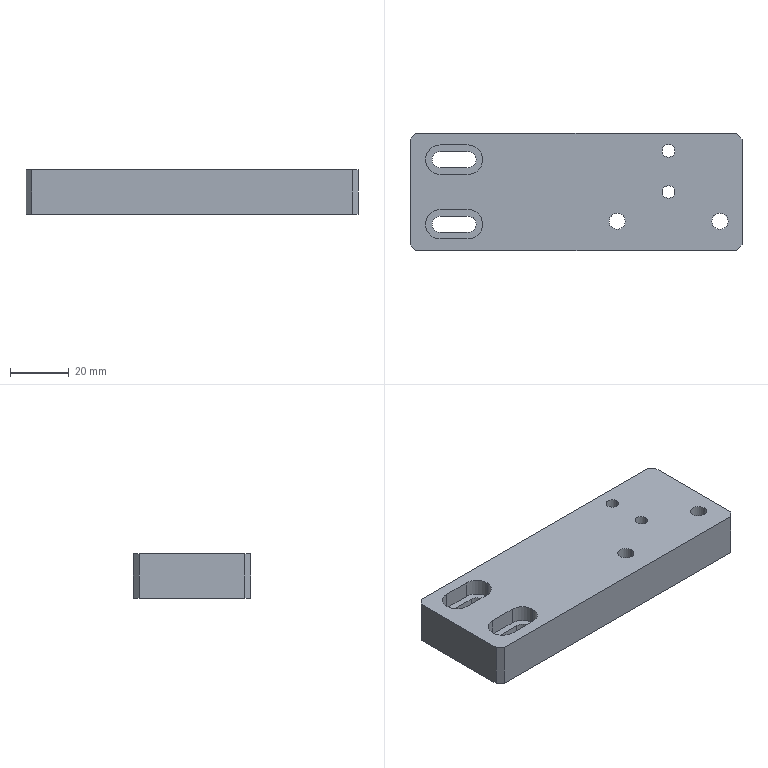Part | STEP file | FBDS-TL-004 | 1 solid | 52 faces | box 113 x 40 x 15 mm | volume 62186 mm3 | cylinder 28 | plane 24 | commonest cylinder face diameters 5.5 x10 10 x10 4.3 x4 8 x4
STEP:
#1=CARTESIAN_POINT('',(35.5,14.,4.6));
#2=VERTEX_POINT('',#1);
#3=CARTESIAN_POINT('',(27.5,14.,4.6));
#4=VERTEX_POINT('',#3);
#5=CARTESIAN_POINT('',(31.5,14.,4.6));
#6=DIRECTION('',(0.,0.,-1.));
#7=DIRECTION('',(-1.,0.,0.));
#8=AXIS2_PLACEMENT_3D('',#5,#6,#7);
#9=CIRCLE('',#8,4.);
#10=EDGE_CURVE('',#2,#4,#9,.T.);
#11=ORIENTED_EDGE('',*,*,#10,.F.);
#12=CARTESIAN_POINT('',(35.5,14.,0.));
#13=VERTEX_POINT('',#12);
#14=CARTESIAN_POINT('',(35.5,14.,0.));
#15=DIRECTION('',(0.,0.,-1.));
#16=VECTOR('',#15,1000.);
#17=LINE('',#14,#16);
#18=EDGE_CURVE('',#2,#13,#17,.T.);
#19=ORIENTED_EDGE('',*,*,#18,.T.);
#20=CARTESIAN_POINT('',(27.5,14.,0.));
#21=VERTEX_POINT('',#20);
#22=CARTESIAN_POINT('',(31.5,14.,0.));
#23=DIRECTION('',(0.,0.,-1.));
#24=DIRECTION('',(-1.,0.,0.));
#25=AXIS2_PLACEMENT_3D('',#22,#23,#24);
#26=CIRCLE('',#25,4.);
#27=EDGE_CURVE('',#13,#21,#26,.T.);
#28=ORIENTED_EDGE('',*,*,#27,.T.);
#29=CARTESIAN_POINT('',(27.5,14.,0.));
#30=DIRECTION('',(0.,0.,-1.));
#31=VECTOR('',#30,1000.);
#32=LINE('',#29,#31);
#33=EDGE_CURVE('',#4,#21,#32,.T.);
#34=ORIENTED_EDGE('',*,*,#33,.F.);
#35=EDGE_LOOP('',(#11,#19,#28,#34));
#36=FACE_OUTER_BOUND('',#35,.T.);
#37=CARTESIAN_POINT('',(31.5,14.,0.));
#38=DIRECTION('',(0.,0.,-1.));
#39=DIRECTION('',(-1.,0.,0.));
#40=AXIS2_PLACEMENT_3D('',#37,#38,#39);
#41=CYLINDRICAL_SURFACE('',#40,4.);
#42=ADVANCED_FACE('',(#36),#41,.F.);
#43=CARTESIAN_POINT('',(33.65,14.,15.));
#44=VERTEX_POINT('',#43);
#45=CARTESIAN_POINT('',(29.35,14.,15.));
#46=VERTEX_POINT('',#45);
#47=CARTESIAN_POINT('',(31.5,14.,15.));
#48=DIRECTION('',(0.,0.,-1.));
#49=DIRECTION('',(-1.,0.,0.));
#50=AXIS2_PLACEMENT_3D('',#47,#48,#49);
#51=CIRCLE('',#50,2.15);
#52=EDGE_CURVE('',#44,#46,#51,.T.);
#53=ORIENTED_EDGE('',*,*,#52,.F.);
#54=CARTESIAN_POINT('',(33.65,14.,4.6));
#55=VERTEX_POINT('',#54);
#56=CARTESIAN_POINT('',(33.65,14.,0.));
#57=DIRECTION('',(0.,0.,-1.));
#58=VECTOR('',#57,1000.);
#59=LINE('',#56,#58);
#60=EDGE_CURVE('',#44,#55,#59,.T.);
#61=ORIENTED_EDGE('',*,*,#60,.T.);
#62=CARTESIAN_POINT('',(29.35,14.,4.6));
#63=VERTEX_POINT('',#62);
#64=CARTESIAN_POINT('',(31.5,14.,4.6));
#65=DIRECTION('',(0.,0.,-1.));
#66=DIRECTION('',(-1.,0.,0.));
#67=AXIS2_PLACEMENT_3D('',#64,#65,#66);
#68=CIRCLE('',#67,2.15);
#69=EDGE_CURVE('',#55,#63,#68,.T.);
#70=ORIENTED_EDGE('',*,*,#69,.T.);
#71=CARTESIAN_POINT('',(29.35,14.,0.));
#72=DIRECTION('',(0.,0.,-1.));
#73=VECTOR('',#72,1000.);
#74=LINE('',#71,#73);
#75=EDGE_CURVE('',#46,#63,#74,.T.);
#76=ORIENTED_EDGE('',*,*,#75,.F.);
#77=EDGE_LOOP('',(#53,#61,#70,#76));
#78=FACE_OUTER_BOUND('',#77,.T.);
#79=CARTESIAN_POINT('',(31.5,14.,0.));
#80=DIRECTION('',(0.,0.,-1.));
#81=DIRECTION('',(-1.,0.,0.));
#82=AXIS2_PLACEMENT_3D('',#79,#80,#81);
#83=CYLINDRICAL_SURFACE('',#82,2.15);
#84=ADVANCED_FACE('',(#78),#83,.F.);
#85=CARTESIAN_POINT('',(35.5,0.,4.6));
#86=VERTEX_POINT('',#85);
#87=CARTESIAN_POINT('',(27.5,0.,4.6));
#88=VERTEX_POINT('',#87);
#89=CARTESIAN_POINT('',(31.5,0.,4.6));
#90=DIRECTION('',(0.,0.,-1.));
#91=DIRECTION('',(-1.,0.,0.));
#92=AXIS2_PLACEMENT_3D('',#89,#90,#91);
#93=CIRCLE('',#92,4.);
#94=EDGE_CURVE('',#86,#88,#93,.T.);
#95=ORIENTED_EDGE('',*,*,#94,.F.);
#96=CARTESIAN_POINT('',(35.5,0.,0.));
#97=VERTEX_POINT('',#96);
#98=CARTESIAN_POINT('',(35.5,0.,0.));
#99=DIRECTION('',(0.,0.,-1.));
#100=VECTOR('',#99,1000.);
#101=LINE('',#98,#100);
#102=EDGE_CURVE('',#86,#97,#101,.T.);
#103=ORIENTED_EDGE('',*,*,#102,.T.);
#104=CARTESIAN_POINT('',(27.5,0.,0.));
#105=VERTEX_POINT('',#104);
#106=CARTESIAN_POINT('',(31.5,0.,0.));
#107=DIRECTION('',(0.,0.,-1.));
#108=DIRECTION('',(-1.,0.,0.));
#109=AXIS2_PLACEMENT_3D('',#106,#107,#108);
#110=CIRCLE('',#109,4.);
#111=EDGE_CURVE('',#97,#105,#110,.T.);
#112=ORIENTED_EDGE('',*,*,#111,.T.);
#113=CARTESIAN_POINT('',(27.5,0.,0.));
#114=DIRECTION('',(0.,0.,-1.));
#115=VECTOR('',#114,1000.);
#116=LINE('',#113,#115);
#117=EDGE_CURVE('',#88,#105,#116,.T.);
#118=ORIENTED_EDGE('',*,*,#117,.F.);
#119=EDGE_LOOP('',(#95,#103,#112,#118));
#120=FACE_OUTER_BOUND('',#119,.T.);
#121=CARTESIAN_POINT('',(31.5,0.,0.));
#122=DIRECTION('',(0.,0.,-1.));
#123=DIRECTION('',(-1.,0.,0.));
#124=AXIS2_PLACEMENT_3D('',#121,#122,#123);
#125=CYLINDRICAL_SURFACE('',#124,4.);
#126=ADVANCED_FACE('',(#120),#125,.F.);
#127=CARTESIAN_POINT('',(33.65,0.,15.));
#128=VERTEX_POINT('',#127);
#129=CARTESIAN_POINT('',(29.35,0.,15.));
#130=VERTEX_POINT('',#129);
#131=CARTESIAN_POINT('',(31.5,0.,15.));
#132=DIRECTION('',(0.,0.,-1.));
#133=DIRECTION('',(-1.,0.,0.));
#134=AXIS2_PLACEMENT_3D('',#131,#132,#133);
#135=CIRCLE('',#134,2.15);
#136=EDGE_CURVE('',#128,#130,#135,.T.);
#137=ORIENTED_EDGE('',*,*,#136,.F.);
#138=CARTESIAN_POINT('',(33.65,0.,4.6));
#139=VERTEX_POINT('',#138);
#140=CARTESIAN_POINT('',(33.65,0.,0.));
#141=DIRECTION('',(0.,0.,-1.));
#142=VECTOR('',#141,1000.);
#143=LINE('',#140,#142);
#144=EDGE_CURVE('',#128,#139,#143,.T.);
#145=ORIENTED_EDGE('',*,*,#144,.T.);
#146=CARTESIAN_POINT('',(29.35,0.,4.6));
#147=VERTEX_POINT('',#146);
#148=CARTESIAN_POINT('',(31.5,0.,4.6));
#149=DIRECTION('',(0.,0.,-1.));
#150=DIRECTION('',(-1.,0.,0.));
#151=AXIS2_PLACEMENT_3D('',#148,#149,#150);
#152=CIRCLE('',#151,2.15);
#153=EDGE_CURVE('',#139,#147,#152,.T.);
#154=ORIENTED_EDGE('',*,*,#153,.T.);
#155=CARTESIAN_POINT('',(29.35,0.,0.));
#156=DIRECTION('',(0.,0.,-1.));
#157=VECTOR('',#156,1000.);
#158=LINE('',#155,#157);
#159=EDGE_CURVE('',#130,#147,#158,.T.);
#160=ORIENTED_EDGE('',*,*,#159,.F.);
#161=EDGE_LOOP('',(#137,#145,#154,#160));
#162=FACE_OUTER_BOUND('',#161,.T.);
#163=CARTESIAN_POINT('',(31.5,0.,0.));
#164=DIRECTION('',(0.,0.,-1.));
#165=DIRECTION('',(-1.,0.,0.));
#166=AXIS2_PLACEMENT_3D('',#163,#164,#165);
#167=CYLINDRICAL_SURFACE('',#166,2.15);
#168=ADVANCED_FACE('',(#162),#167,.F.);
#169=CARTESIAN_POINT('',(19.,-10.,5.7));
#170=VERTEX_POINT('',#169);
#171=CARTESIAN_POINT('',(9.,-10.,5.7));
#172=VERTEX_POINT('',#171);
#173=CARTESIAN_POINT('',(14.,-10.,5.7));
#174=DIRECTION('',(0.,0.,-1.));
#175=DIRECTION('',(-1.,0.,0.));
#176=AXIS2_PLACEMENT_3D('',#173,#174,#175);
#177=CIRCLE('',#176,5.);
#178=EDGE_CURVE('',#170,#172,#177,.T.);
#179=ORIENTED_EDGE('',*,*,#178,.F.);
#180=CARTESIAN_POINT('',(19.,-10.,0.));
#181=VERTEX_POINT('',#180);
#182=CARTESIAN_POINT('',(19.,-10.,0.));
#183=DIRECTION('',(0.,0.,-1.));
#184=VECTOR('',#183,1000.);
#185=LINE('',#182,#184);
#186=EDGE_CURVE('',#170,#181,#185,.T.);
#187=ORIENTED_EDGE('',*,*,#186,.T.);
#188=CARTESIAN_POINT('',(9.,-10.,0.));
#189=VERTEX_POINT('',#188);
#190=CARTESIAN_POINT('',(14.,-10.,0.));
#191=DIRECTION('',(0.,0.,-1.));
#192=DIRECTION('',(-1.,0.,0.));
#193=AXIS2_PLACEMENT_3D('',#190,#191,#192);
#194=CIRCLE('',#193,5.);
#195=EDGE_CURVE('',#181,#189,#194,.T.);
#196=ORIENTED_EDGE('',*,*,#195,.T.);
#197=CARTESIAN_POINT('',(9.,-10.,0.));
#198=DIRECTION('',(0.,0.,-1.));
#199=VECTOR('',#198,1000.);
#200=LINE('',#197,#199);
#201=EDGE_CURVE('',#172,#189,#200,.T.);
#202=ORIENTED_EDGE('',*,*,#201,.F.);
#203=EDGE_LOOP('',(#179,#187,#196,#202));
#204=FACE_OUTER_BOUND('',#203,.T.);
#205=CARTESIAN_POINT('',(14.,-10.,0.));
#206=DIRECTION('',(0.,0.,-1.));
#207=DIRECTION('',(-1.,0.,0.));
#208=AXIS2_PLACEMENT_3D('',#205,#206,#207);
#209=CYLINDRICAL_SURFACE('',#208,5.);
#210=ADVANCED_FACE('',(#204),#209,.F.);
#211=CARTESIAN_POINT('',(16.75,-10.,15.));
#212=VERTEX_POINT('',#211);
#213=CARTESIAN_POINT('',(11.25,-10.,15.));
#214=VERTEX_POINT('',#213);
#215=CARTESIAN_POINT('',(14.,-10.,15.));
#216=DIRECTION('',(0.,0.,-1.));
#217=DIRECTION('',(-1.,0.,0.));
#218=AXIS2_PLACEMENT_3D('',#215,#216,#217);
#219=CIRCLE('',#218,2.75);
#220=EDGE_CURVE('',#212,#214,#219,.T.);
#221=ORIENTED_EDGE('',*,*,#220,.F.);
#222=CARTESIAN_POINT('',(16.75,-10.,5.7));
#223=VERTEX_POINT('',#222);
#224=CARTESIAN_POINT('',(16.75,-10.,0.));
#225=DIRECTION('',(0.,0.,-1.));
#226=VECTOR('',#225,1000.);
#227=LINE('',#224,#226);
#228=EDGE_CURVE('',#212,#223,#227,.T.);
#229=ORIENTED_EDGE('',*,*,#228,.T.);
#230=CARTESIAN_POINT('',(11.25,-10.,5.7));
#231=VERTEX_POINT('',#230);
#232=CARTESIAN_POINT('',(14.,-10.,5.7));
#233=DIRECTION('',(0.,0.,-1.));
#234=DIRECTION('',(-1.,0.,0.));
#235=AXIS2_PLACEMENT_3D('',#232,#233,#234);
#236=CIRCLE('',#235,2.75);
#237=EDGE_CURVE('',#223,#231,#236,.T.);
#238=ORIENTED_EDGE('',*,*,#237,.T.);
#239=CARTESIAN_POINT('',(11.25,-10.,0.));
#240=DIRECTION('',(0.,0.,-1.));
#241=VECTOR('',#240,1000.);
#242=LINE('',#239,#241);
#243=EDGE_CURVE('',#214,#231,#242,.T.);
#244=ORIENTED_EDGE('',*,*,#243,.F.);
#245=EDGE_LOOP('',(#221,#229,#238,#244));
#246=FACE_OUTER_BOUND('',#245,.T.);
#247=CARTESIAN_POINT('',(14.,-10.,0.));
#248=DIRECTION('',(0.,0.,-1.));
#249=DIRECTION('',(-1.,0.,0.));
#250=AXIS2_PLACEMENT_3D('',#247,#248,#249);
#251=CYLINDRICAL_SURFACE('',#250,2.75);
#252=ADVANCED_FACE('',(#246),#251,.F.);
#253=CARTESIAN_POINT('',(54.,-10.,5.7));
#254=VERTEX_POINT('',#253);
#255=CARTESIAN_POINT('',(44.,-10.,5.7));
#256=VERTEX_POINT('',#255);
#257=CARTESIAN_POINT('',(49.,-10.,5.7));
#258=DIRECTION('',(0.,0.,-1.));
#259=DIRECTION('',(-1.,0.,0.));
#260=AXIS2_PLACEMENT_3D('',#257,#258,#259);
#261=CIRCLE('',#260,5.);
#262=EDGE_CURVE('',#254,#256,#261,.T.);
#263=ORIENTED_EDGE('',*,*,#262,.F.);
#264=CARTESIAN_POINT('',(54.,-10.,0.));
#265=VERTEX_POINT('',#264);
#266=CARTESIAN_POINT('',(54.,-10.,0.));
#267=DIRECTION('',(0.,0.,-1.));
#268=VECTOR('',#267,1000.);
#269=LINE('',#266,#268);
#270=EDGE_CURVE('',#254,#265,#269,.T.);
#271=ORIENTED_EDGE('',*,*,#270,.T.);
#272=CARTESIAN_POINT('',(44.,-10.,0.));
#273=VERTEX_POINT('',#272);
#274=CARTESIAN_POINT('',(49.,-10.,0.));
#275=DIRECTION('',(0.,0.,-1.));
#276=DIRECTION('',(-1.,0.,0.));
#277=AXIS2_PLACEMENT_3D('',#274,#275,#276);
#278=CIRCLE('',#277,5.);
#279=EDGE_CURVE('',#265,#273,#278,.T.);
#280=ORIENTED_EDGE('',*,*,#279,.T.);
#281=CARTESIAN_POINT('',(44.,-10.,0.));
#282=DIRECTION('',(0.,0.,-1.));
#283=VECTOR('',#282,1000.);
#284=LINE('',#281,#283);
#285=EDGE_CURVE('',#256,#273,#284,.T.);
#286=ORIENTED_EDGE('',*,*,#285,.F.);
#287=EDGE_LOOP('',(#263,#271,#280,#286));
#288=FACE_OUTER_BOUND('',#287,.T.);
#289=CARTESIAN_POINT('',(49.,-10.,0.));
#290=DIRECTION('',(0.,0.,-1.));
#291=DIRECTION('',(-1.,0.,0.));
#292=AXIS2_PLACEMENT_3D('',#289,#290,#291);
#293=CYLINDRICAL_SURFACE('',#292,5.);
#294=ADVANCED_FACE('',(#288),#293,.F.);
#295=CARTESIAN_POINT('',(51.75,-10.,15.));
#296=VERTEX_POINT('',#295);
#297=CARTESIAN_POINT('',(46.25,-10.,15.));
#298=VERTEX_POINT('',#297);
#299=CARTESIAN_POINT('',(49.,-10.,15.));
#300=DIRECTION('',(0.,0.,-1.));
#301=DIRECTION('',(-1.,0.,0.));
#302=AXIS2_PLACEMENT_3D('',#299,#300,#301);
#303=CIRCLE('',#302,2.75);
#304=EDGE_CURVE('',#296,#298,#303,.T.);
#305=ORIENTED_EDGE('',*,*,#304,.F.);
#306=CARTESIAN_POINT('',(51.75,-10.,5.7));
#307=VERTEX_POINT('',#306);
#308=CARTESIAN_POINT('',(51.75,-10.,0.));
#309=DIRECTION('',(0.,0.,-1.));
#310=VECTOR('',#309,1000.);
#311=LINE('',#308,#310);
#312=EDGE_CURVE('',#296,#307,#311,.T.);
#313=ORIENTED_EDGE('',*,*,#312,.T.);
#314=CARTESIAN_POINT('',(46.25,-10.,5.7));
#315=VERTEX_POINT('',#314);
#316=CARTESIAN_POINT('',(49.,-10.,5.7));
#317=DIRECTION('',(0.,0.,-1.));
#318=DIRECTION('',(-1.,0.,0.));
#319=AXIS2_PLACEMENT_3D('',#316,#317,#318);
#320=CIRCLE('',#319,2.75);
#321=EDGE_CURVE('',#307,#315,#320,.T.);
#322=ORIENTED_EDGE('',*,*,#321,.T.);
#323=CARTESIAN_POINT('',(46.25,-10.,0.));
#324=DIRECTION('',(0.,0.,-1.));
#325=VECTOR('',#324,1000.);
#326=LINE('',#323,#325);
#327=EDGE_CURVE('',#298,#315,#326,.T.);
#328=ORIENTED_EDGE('',*,*,#327,.F.);
#329=EDGE_LOOP('',(#305,#313,#322,#328));
#330=FACE_OUTER_BOUND('',#329,.T.);
#331=CARTESIAN_POINT('',(49.,-10.,0.));
#332=DIRECTION('',(0.,0.,-1.));
#333=DIRECTION('',(-1.,0.,0.));
#334=AXIS2_PLACEMENT_3D('',#331,#332,#333);
#335=CYLINDRICAL_SURFACE('',#334,2.75);
#336=ADVANCED_FACE('',(#330),#335,.F.);
#337=CARTESIAN_POINT('',(-31.75,11.,9.3));
#338=VERTEX_POINT('',#337);
#339=CARTESIAN_POINT('',(-36.75,16.,9.3));
#340=VERTEX_POINT('',#339);
#341=CARTESIAN_POINT('',(-36.75,11.,9.3));
#342=DIRECTION('',(0.,0.,1.));
#343=DIRECTION('',(1.,0.,0.));
#344=AXIS2_PLACEMENT_3D('',#341,#342,#343);
#345=CIRCLE('',#344,5.);
#346=EDGE_CURVE('',#338,#340,#345,.T.);
#347=ORIENTED_EDGE('',*,*,#346,.F.);
#348=CARTESIAN_POINT('',(-31.75,11.,15.));
#349=VERTEX_POINT('',#348);
#350=CARTESIAN_POINT('',(-31.75,11.,15.));
#351=DIRECTION('',(0.,0.,1.));
#352=VECTOR('',#351,1000.);
#353=LINE('',#350,#352);
#354=EDGE_CURVE('',#338,#349,#353,.T.);
#355=ORIENTED_EDGE('',*,*,#354,.T.);
#356=CARTESIAN_POINT('',(-36.75,16.,15.));
#357=VERTEX_POINT('',#356);
#358=CARTESIAN_POINT('',(-36.75,11.,15.));
#359=DIRECTION('',(0.,0.,1.));
#360=DIRECTION('',(1.,0.,0.));
#361=AXIS2_PLACEMENT_3D('',#358,#359,#360);
#362=CIRCLE('',#361,5.);
#363=EDGE_CURVE('',#349,#357,#362,.T.);
#364=ORIENTED_EDGE('',*,*,#363,.T.);
#365=CARTESIAN_POINT('',(-36.75,16.,15.));
#366=DIRECTION('',(0.,0.,1.));
#367=VECTOR('',#366,1000.);
#368=LINE('',#365,#367);
#369=EDGE_CURVE('',#340,#357,#368,.T.);
#370=ORIENTED_EDGE('',*,*,#369,.F.);
#371=EDGE_LOOP('',(#347,#355,#364,#370));
#372=FACE_OUTER_BOUND('',#371,.T.);
#373=CARTESIAN_POINT('',(-36.75,11.,15.));
#374=DIRECTION('',(0.,0.,1.));
#375=DIRECTION('',(1.,0.,0.));
#376=AXIS2_PLACEMENT_3D('',#373,#374,#375);
#377=CYLINDRICAL_SURFACE('',#376,5.);
#378=ADVANCED_FACE('',(#372),#377,.F.);
#379=CARTESIAN_POINT('',(-34.,11.,0.));
#380=VERTEX_POINT('',#379);
#381=CARTESIAN_POINT('',(-36.75,13.75,0.));
#382=VERTEX_POINT('',#381);
#383=CARTESIAN_POINT('',(-36.75,11.,0.));
#384=DIRECTION('',(0.,0.,1.));
#385=DIRECTION('',(1.,0.,0.));
#386=AXIS2_PLACEMENT_3D('',#383,#384,#385);
#387=CIRCLE('',#386,2.75);
#388=EDGE_CURVE('',#380,#382,#387,.T.);
#389=ORIENTED_EDGE('',*,*,#388,.F.);
#390=CARTESIAN_POINT('',(-34.,11.,9.3));
#391=VERTEX_POINT('',#390);
#392=CARTESIAN_POINT('',(-34.,11.,15.));
#393=DIRECTION('',(0.,0.,1.));
#394=VECTOR('',#393,1000.);
#395=LINE('',#392,#394);
#396=EDGE_CURVE('',#380,#391,#395,.T.);
#397=ORIENTED_EDGE('',*,*,#396,.T.);
#398=CARTESIAN_POINT('',(-36.75,13.75,9.3));
#399=VERTEX_POINT('',#398);
#400=CARTESIAN_POINT('',(-36.75,11.,9.3));
#401=DIRECTION('',(0.,0.,1.));
#402=DIRECTION('',(1.,0.,0.));
#403=AXIS2_PLACEMENT_3D('',#400,#401,#402);
#404=CIRCLE('',#403,2.75);
#405=EDGE_CURVE('',#391,#399,#404,.T.);
#406=ORIENTED_EDGE('',*,*,#405,.T.);
#407=CARTESIAN_POINT('',(-36.75,13.75,15.));
#408=DIRECTION('',(0.,0.,1.));
#409=VECTOR('',#408,1000.);
#410=LINE('',#407,#409);
#411=EDGE_CURVE('',#382,#399,#410,.T.);
#412=ORIENTED_EDGE('',*,*,#411,.F.);
#413=EDGE_LOOP('',(#389,#397,#406,#412));
#414=FACE_OUTER_BOUND('',#413,.T.);
#415=CARTESIAN_POINT('',(-36.75,11.,15.));
#416=DIRECTION('',(0.,0.,1.));
#417=DIRECTION('',(1.,0.,0.));
#418=AXIS2_PLACEMENT_3D('',#415,#416,#417);
#419=CYLINDRICAL_SURFACE('',#418,2.75);
#420=ADVANCED_FACE('',(#414),#419,.F.);
#421=CARTESIAN_POINT('',(-31.75,-11.,9.3));
#422=VERTEX_POINT('',#421);
#423=CARTESIAN_POINT('',(-36.75,-6.,9.3));
#424=VERTEX_POINT('',#423);
#425=CARTESIAN_POINT('',(-36.75,-11.,9.3));
#426=DIRECTION('',(0.,0.,1.));
#427=DIRECTION('',(1.,0.,0.));
#428=AXIS2_PLACEMENT_3D('',#425,#426,#427);
#429=CIRCLE('',#428,5.);
#430=EDGE_CURVE('',#422,#424,#429,.T.);
#431=ORIENTED_EDGE('',*,*,#430,.F.);
#432=CARTESIAN_POINT('',(-31.75,-11.,15.));
#433=VERTEX_POINT('',#432);
#434=CARTESIAN_POINT('',(-31.75,-11.,15.));
#435=DIRECTION('',(0.,0.,1.));
#436=VECTOR('',#435,1000.);
#437=LINE('',#434,#436);
#438=EDGE_CURVE('',#422,#433,#437,.T.);
#439=ORIENTED_EDGE('',*,*,#438,.T.);
#440=CARTESIAN_POINT('',(-36.75,-6.,15.));
#441=VERTEX_POINT('',#440);
#442=CARTESIAN_POINT('',(-36.75,-11.,15.));
#443=DIRECTION('',(0.,0.,1.));
#444=DIRECTION('',(1.,0.,0.));
#445=AXIS2_PLACEMENT_3D('',#442,#443,#444);
#446=CIRCLE('',#445,5.);
#447=EDGE_CURVE('',#433,#441,#446,.T.);
#448=ORIENTED_EDGE('',*,*,#447,.T.);
#449=CARTESIAN_POINT('',(-36.75,-6.,15.));
#450=DIRECTION('',(0.,0.,1.));
#451=VECTOR('',#450,1000.);
#452=LINE('',#449,#451);
#453=EDGE_CURVE('',#424,#441,#452,.T.);
#454=ORIENTED_EDGE('',*,*,#453,.F.);
#455=EDGE_LOOP('',(#431,#439,#448,#454));
#456=FACE_OUTER_BOUND('',#455,.T.);
#457=CARTESIAN_POINT('',(-36.75,-11.,15.));
#458=DIRECTION('',(0.,0.,1.));
#459=DIRECTION('',(1.,0.,0.));
#460=AXIS2_PLACEMENT_3D('',#457,#458,#459);
#461=CYLINDRICAL_SURFACE('',#460,5.);
#462=ADVANCED_FACE('',(#456),#461,.F.);
#463=CARTESIAN_POINT('',(-34.,-11.,0.));
#464=VERTEX_POINT('',#463);
#465=CARTESIAN_POINT('',(-36.75,-8.25,0.));
#466=VERTEX_POINT('',#465);
#467=CARTESIAN_POINT('',(-36.75,-11.,0.));
#468=DIRECTION('',(0.,0.,1.));
#469=DIRECTION('',(1.,0.,0.));
#470=AXIS2_PLACEMENT_3D('',#467,#468,#469);
#471=CIRCLE('',#470,2.75);
#472=EDGE_CURVE('',#464,#466,#471,.T.);
#473=ORIENTED_EDGE('',*,*,#472,.F.);
#474=CARTESIAN_POINT('',(-34.,-11.,9.3));
#475=VERTEX_POINT('',#474);
#476=CARTESIAN_POINT('',(-34.,-11.,15.));
#477=DIRECTION('',(0.,0.,1.));
#478=VECTOR('',#477,1000.);
#479=LINE('',#476,#478);
#480=EDGE_CURVE('',#464,#475,#479,.T.);
#481=ORIENTED_EDGE('',*,*,#480,.T.);
#482=CARTESIAN_POINT('',(-36.75,-8.25,9.3));
#483=VERTEX_POINT('',#482);
#484=CARTESIAN_POINT('',(-36.75,-11.,9.3));
#485=DIRECTION('',(0.,0.,1.));
#486=DIRECTION('',(1.,0.,0.));
#487=AXIS2_PLACEMENT_3D('',#484,#485,#486);
#488=CIRCLE('',#487,2.75);
#489=EDGE_CURVE('',#475,#483,#488,.T.);
#490=ORIENTED_EDGE('',*,*,#489,.T.);
#491=CARTESIAN_POINT('',(-36.75,-8.25,15.));
#492=DIRECTION('',(0.,0.,1.));
#493=VECTOR('',#492,1000.);
#494=LINE('',#491,#493);
#495=EDGE_CURVE('',#466,#483,#494,.T.);
#496=ORIENTED_EDGE('',*,*,#495,.F.);
#497=EDGE_LOOP('',(#473,#481,#490,#496));
#498=FACE_OUTER_BOUND('',#497,.T.);
#499=CARTESIAN_POINT('',(-36.75,-11.,15.));
#500=DIRECTION('',(0.,0.,1.));
#501=DIRECTION('',(1.,0.,0.));
#502=AXIS2_PLACEMENT_3D('',#499,#500,#501);
#503=CYLINDRICAL_SURFACE('',#502,2.75);
#504=ADVANCED_FACE('',(#498),#503,.F.);
#505=CARTESIAN_POINT('',(31.5,14.,15.));
#506=DIRECTION('',(0.,0.,-1.));
#507=DIRECTION('',(-1.,0.,0.));
#508=AXIS2_PLACEMENT_3D('',#505,#506,#507);
#509=CIRCLE('',#508,2.15);
#510=EDGE_CURVE('',#46,#44,#509,.T.);
#511=ORIENTED_EDGE('',*,*,#510,.T.);
#512=ORIENTED_EDGE('',*,*,#52,.T.);
#513=EDGE_LOOP('',(#511,#512));
#514=FACE_BOUND('',#513,.T.);
#515=CARTESIAN_POINT('',(31.5,0.,15.));
#516=DIRECTION('',(0.,0.,-1.));
#517=DIRECTION('',(-1.,0.,0.));
#518=AXIS2_PLACEMENT_3D('',#515,#516,#517);
#519=CIRCLE('',#518,2.15);
#520=EDGE_CURVE('',#130,#128,#519,.T.);
#521=ORIENTED_EDGE('',*,*,#520,.T.);
#522=ORIENTED_EDGE('',*,*,#136,.T.);
#523=EDGE_LOOP('',(#521,#522));
#524=FACE_BOUND('',#523,.T.);
#525=CARTESIAN_POINT('',(14.,-10.,15.));
#526=DIRECTION('',(0.,0.,-1.));
#527=DIRECTION('',(-1.,0.,0.));
#528=AXIS2_PLACEMENT_3D('',#525,#526,#527);
#529=CIRCLE('',#528,2.75);
#530=EDGE_CURVE('',#214,#212,#529,.T.);
#531=ORIENTED_EDGE('',*,*,#530,.T.);
#532=ORIENTED_EDGE('',*,*,#220,.T.);
#533=EDGE_LOOP('',(#531,#532));
#534=FACE_BOUND('',#533,.T.);
#535=CARTESIAN_POINT('',(49.,-10.,15.));
#536=DIRECTION('',(0.,0.,-1.));
#537=DIRECTION('',(-1.,0.,0.));
#538=AXIS2_PLACEMENT_3D('',#535,#536,#537);
#539=CIRCLE('',#538,2.75);
#540=EDGE_CURVE('',#298,#296,#539,.T.);
#541=ORIENTED_EDGE('',*,*,#540,.T.);
#542=ORIENTED_EDGE('',*,*,#304,.T.);
#543=EDGE_LOOP('',(#541,#542));
#544=FACE_BOUND('',#543,.T.);
#545=CARTESIAN_POINT('',(56.5,-18.,15.));
#546=VERTEX_POINT('',#545);
#547=CARTESIAN_POINT('',(56.5,18.,15.));
#548=VERTEX_POINT('',#547);
#549=CARTESIAN_POINT('',(56.5,-20.,15.));
#550=DIRECTION('',(0.,1.,0.));
#551=VECTOR('',#550,1000.);
#552=LINE('',#549,#551);
#553=EDGE_CURVE('',#546,#548,#552,.T.);
#554=ORIENTED_EDGE('',*,*,#553,.T.);
#555=CARTESIAN_POINT('',(54.5,20.,15.));
#556=VERTEX_POINT('',#555);
#557=CARTESIAN_POINT('',(54.5,20.,15.));
#558=DIRECTION('',(-0.7071,0.7071,0.));
#559=VECTOR('',#558,1000.);
#560=LINE('',#557,#559);
#561=EDGE_CURVE('',#548,#556,#560,.T.);
#562=ORIENTED_EDGE('',*,*,#561,.T.);
#563=CARTESIAN_POINT('',(-54.5,20.,15.));
#564=VERTEX_POINT('',#563);
#565=CARTESIAN_POINT('',(-56.5,20.,15.));
#566=DIRECTION('',(-1.,0.,0.));
#567=VECTOR('',#566,1000.);
#568=LINE('',#565,#567);
#569=EDGE_CURVE('',#556,#564,#568,.T.);
#570=ORIENTED_EDGE('',*,*,#569,.T.);
#571=CARTESIAN_POINT('',(-56.5,18.,15.));
#572=VERTEX_POINT('',#571);
#573=CARTESIAN_POINT('',(-56.5,18.,15.));
#574=DIRECTION('',(-0.7071,-0.7071,0.));
#575=VECTOR('',#574,1000.);
#576=LINE('',#573,#575);
#577=EDGE_CURVE('',#564,#572,#576,.T.);
#578=ORIENTED_EDGE('',*,*,#577,.T.);
#579=CARTESIAN_POINT('',(-56.5,-18.,15.));
#580=VERTEX_POINT('',#579);
#581=CARTESIAN_POINT('',(-56.5,-20.,15.));
#582=DIRECTION('',(0.,-1.,0.));
#583=VECTOR('',#582,1000.);
#584=LINE('',#581,#583);
#585=EDGE_CURVE('',#572,#580,#584,.T.);
#586=ORIENTED_EDGE('',*,*,#585,.T.);
#587=CARTESIAN_POINT('',(-54.5,-20.,15.));
#588=VERTEX_POINT('',#587);
#589=CARTESIAN_POINT('',(-54.5,-20.,15.));
#590=DIRECTION('',(0.7071,-0.7071,0.));
#591=VECTOR('',#590,1000.);
#592=LINE('',#589,#591);
#593=EDGE_CURVE('',#580,#588,#592,.T.);
#594=ORIENTED_EDGE('',*,*,#593,.T.);
#595=CARTESIAN_POINT('',(54.5,-20.,15.));
#596=VERTEX_POINT('',#595);
#597=CARTESIAN_POINT('',(-56.5,-20.,15.));
#598=DIRECTION('',(1.,0.,0.));
#599=VECTOR('',#598,1000.);
#600=LINE('',#597,#599);
#601=EDGE_CURVE('',#588,#596,#600,.T.);
#602=ORIENTED_EDGE('',*,*,#601,.T.);
#603=CARTESIAN_POINT('',(56.5,-18.,15.));
#604=DIRECTION('',(0.7071,0.7071,0.));
#605=VECTOR('',#604,1000.);
#606=LINE('',#603,#605);
#607=EDGE_CURVE('',#596,#546,#606,.T.);
#608=ORIENTED_EDGE('',*,*,#607,.T.);
#609=EDGE_LOOP('',(#554,#562,#570,#578,#586,#594,#602,#608));
#610=FACE_OUTER_BOUND('',#609,.T.);
#611=CARTESIAN_POINT('',(-46.25,-6.,15.));
#612=VERTEX_POINT('',#611);
#613=CARTESIAN_POINT('',(-46.25,-16.,15.));
#614=VERTEX_POINT('',#613);
#615=CARTESIAN_POINT('',(-46.25,-11.,15.));
#616=DIRECTION('',(0.,0.,1.));
#617=DIRECTION('',(1.,0.,0.));
#618=AXIS2_PLACEMENT_3D('',#615,#616,#617);
#619=CIRCLE('',#618,5.);
#620=EDGE_CURVE('',#612,#614,#619,.T.);
#621=ORIENTED_EDGE('',*,*,#620,.F.);
#622=CARTESIAN_POINT('',(-46.25,-6.,15.));
#623=DIRECTION('',(1.,0.,0.));
#624=VECTOR('',#623,1000.);
#625=LINE('',#622,#624);
#626=EDGE_CURVE('',#612,#441,#625,.T.);
#627=ORIENTED_EDGE('',*,*,#626,.T.);
#628=ORIENTED_EDGE('',*,*,#447,.F.);
#629=CARTESIAN_POINT('',(-36.75,-16.,15.));
#630=VERTEX_POINT('',#629);
#631=CARTESIAN_POINT('',(-36.75,-11.,15.));
#632=DIRECTION('',(0.,0.,1.));
#633=DIRECTION('',(1.,0.,0.));
#634=AXIS2_PLACEMENT_3D('',#631,#632,#633);
#635=CIRCLE('',#634,5.);
#636=EDGE_CURVE('',#630,#433,#635,.T.);
#637=ORIENTED_EDGE('',*,*,#636,.F.);
#638=CARTESIAN_POINT('',(-46.25,-16.,15.));
#639=DIRECTION('',(1.,0.,0.));
#640=VECTOR('',#639,1000.);
#641=LINE('',#638,#640);
#642=EDGE_CURVE('',#614,#630,#641,.T.);
#643=ORIENTED_EDGE('',*,*,#642,.F.);
#644=EDGE_LOOP('',(#621,#627,#628,#637,#643));
#645=FACE_BOUND('',#644,.T.);
#646=CARTESIAN_POINT('',(-36.75,6.,15.));
#647=VERTEX_POINT('',#646);
#648=CARTESIAN_POINT('',(-36.75,11.,15.));
#649=DIRECTION('',(0.,0.,1.));
#650=DIRECTION('',(1.,0.,0.));
#651=AXIS2_PLACEMENT_3D('',#648,#649,#650);
#652=CIRCLE('',#651,5.);
#653=EDGE_CURVE('',#647,#349,#652,.T.);
#654=ORIENTED_EDGE('',*,*,#653,.F.);
#655=CARTESIAN_POINT('',(-46.25,6.,15.));
#656=VERTEX_POINT('',#655);
#657=CARTESIAN_POINT('',(-46.25,6.,15.));
#658=DIRECTION('',(1.,0.,0.));
#659=VECTOR('',#658,1000.);
#660=LINE('',#657,#659);
#661=EDGE_CURVE('',#656,#647,#660,.T.);
#662=ORIENTED_EDGE('',*,*,#661,.F.);
#663=CARTESIAN_POINT('',(-46.25,16.,15.));
#664=VERTEX_POINT('',#663);
#665=CARTESIAN_POINT('',(-46.25,11.,15.));
#666=DIRECTION('',(0.,0.,1.));
#667=DIRECTION('',(1.,0.,0.));
#668=AXIS2_PLACEMENT_3D('',#665,#666,#667);
#669=CIRCLE('',#668,5.);
#670=EDGE_CURVE('',#664,#656,#669,.T.);
#671=ORIENTED_EDGE('',*,*,#670,.F.);
#672=CARTESIAN_POINT('',(-46.25,16.,15.));
#673=DIRECTION('',(1.,0.,0.));
#674=VECTOR('',#673,1000.);
#675=LINE('',#672,#674);
#676=EDGE_CURVE('',#664,#357,#675,.T.);
#677=ORIENTED_EDGE('',*,*,#676,.T.);
#678=ORIENTED_EDGE('',*,*,#363,.F.);
#679=EDGE_LOOP('',(#654,#662,#671,#677,#678));
#680=FACE_BOUND('',#679,.T.);
#681=CARTESIAN_POINT('',(0.,0.,15.));
#682=DIRECTION('',(0.,0.,-1.));
#683=DIRECTION('',(-1.,0.,0.));
#684=AXIS2_PLACEMENT_3D('',#681,#682,#683);
#685=PLANE('',#684);
#686=ADVANCED_FACE('',(#514,#524,#534,#544,#610,#645,#680),#685,.F.);
#687=CARTESIAN_POINT('',(31.5,14.,0.));
#688=DIRECTION('',(0.,0.,-1.));
#689=DIRECTION('',(-1.,0.,0.));
#690=AXIS2_PLACEMENT_3D('',#687,#688,#689);
#691=CIRCLE('',#690,4.);
#692=EDGE_CURVE('',#21,#13,#691,.T.);
#693=ORIENTED_EDGE('',*,*,#692,.F.);
#694=ORIENTED_EDGE('',*,*,#27,.F.);
#695=EDGE_LOOP('',(#693,#694));
#696=FACE_BOUND('',#695,.T.);
#697=CARTESIAN_POINT('',(31.5,0.,0.));
#698=DIRECTION('',(0.,0.,-1.));
#699=DIRECTION('',(-1.,0.,0.));
#700=AXIS2_PLACEMENT_3D('',#697,#698,#699);
#701=CIRCLE('',#700,4.);
#702=EDGE_CURVE('',#105,#97,#701,.T.);
#703=ORIENTED_EDGE('',*,*,#702,.F.);
#704=ORIENTED_EDGE('',*,*,#111,.F.);
#705=EDGE_LOOP('',(#703,#704));
#706=FACE_BOUND('',#705,.T.);
#707=CARTESIAN_POINT('',(14.,-10.,0.));
#708=DIRECTION('',(0.,0.,-1.));
#709=DIRECTION('',(-1.,0.,0.));
#710=AXIS2_PLACEMENT_3D('',#707,#708,#709);
#711=CIRCLE('',#710,5.);
#712=EDGE_CURVE('',#189,#181,#711,.T.);
#713=ORIENTED_EDGE('',*,*,#712,.F.);
#714=ORIENTED_EDGE('',*,*,#195,.F.);
#715=EDGE_LOOP('',(#713,#714));
#716=FACE_BOUND('',#715,.T.);
#717=CARTESIAN_POINT('',(49.,-10.,0.));
#718=DIRECTION('',(0.,0.,-1.));
#719=DIRECTION('',(-1.,0.,0.));
#720=AXIS2_PLACEMENT_3D('',#717,#718,#719);
#721=CIRCLE('',#720,5.);
#722=EDGE_CURVE('',#273,#265,#721,.T.);
#723=ORIENTED_EDGE('',*,*,#722,.F.);
#724=ORIENTED_EDGE('',*,*,#279,.F.);
#725=EDGE_LOOP('',(#723,#724));
#726=FACE_BOUND('',#725,.T.);
#727=CARTESIAN_POINT('',(54.5,20.,0.));
#728=VERTEX_POINT('',#727);
#729=CARTESIAN_POINT('',(-54.5,20.,0.));
#730=VERTEX_POINT('',#729);
#731=CARTESIAN_POINT('',(-56.5,20.,0.));
#732=DIRECTION('',(-1.,0.,0.));
#733=VECTOR('',#732,1000.);
#734=LINE('',#731,#733);
#735=EDGE_CURVE('',#728,#730,#734,.T.);
#736=ORIENTED_EDGE('',*,*,#735,.F.);
#737=CARTESIAN_POINT('',(56.5,18.,0.));
#738=VERTEX_POINT('',#737);
#739=CARTESIAN_POINT('',(37.25,37.25,0.));
#740=DIRECTION('',(0.7071,-0.7071,0.));
#741=VECTOR('',#740,1000.);
#742=LINE('',#739,#741);
#743=EDGE_CURVE('',#728,#738,#742,.T.);
#744=ORIENTED_EDGE('',*,*,#743,.T.);
#745=CARTESIAN_POINT('',(56.5,-18.,0.));
#746=VERTEX_POINT('',#745);
#747=CARTESIAN_POINT('',(56.5,-20.,0.));
#748=DIRECTION('',(0.,1.,0.));
#749=VECTOR('',#748,1000.);
#750=LINE('',#747,#749);
#751=EDGE_CURVE('',#746,#738,#750,.T.);
#752=ORIENTED_EDGE('',*,*,#751,.F.);
#753=CARTESIAN_POINT('',(54.5,-20.,0.));
#754=VERTEX_POINT('',#753);
#755=CARTESIAN_POINT('',(37.25,-37.25,0.));
#756=DIRECTION('',(-0.7071,-0.7071,0.));
#757=VECTOR('',#756,1000.);
#758=LINE('',#755,#757);
#759=EDGE_CURVE('',#746,#754,#758,.T.);
#760=ORIENTED_EDGE('',*,*,#759,.T.);
#761=CARTESIAN_POINT('',(-54.5,-20.,0.));
#762=VERTEX_POINT('',#761);
#763=CARTESIAN_POINT('',(-56.5,-20.,0.));
#764=DIRECTION('',(1.,0.,0.));
#765=VECTOR('',#764,1000.);
#766=LINE('',#763,#765);
#767=EDGE_CURVE('',#762,#754,#766,.T.);
#768=ORIENTED_EDGE('',*,*,#767,.F.);
#769=CARTESIAN_POINT('',(-56.5,-18.,0.));
#770=VERTEX_POINT('',#769);
#771=CARTESIAN_POINT('',(-37.25,-37.25,0.));
#772=DIRECTION('',(-0.7071,0.7071,0.));
#773=VECTOR('',#772,1000.);
#774=LINE('',#771,#773);
#775=EDGE_CURVE('',#762,#770,#774,.T.);
#776=ORIENTED_EDGE('',*,*,#775,.T.);
#777=CARTESIAN_POINT('',(-56.5,18.,0.));
#778=VERTEX_POINT('',#777);
#779=CARTESIAN_POINT('',(-56.5,-20.,0.));
#780=DIRECTION('',(0.,-1.,0.));
#781=VECTOR('',#780,1000.);
#782=LINE('',#779,#781);
#783=EDGE_CURVE('',#778,#770,#782,.T.);
#784=ORIENTED_EDGE('',*,*,#783,.F.);
#785=CARTESIAN_POINT('',(-37.25,37.25,0.));
#786=DIRECTION('',(0.7071,0.7071,0.));
#787=VECTOR('',#786,1000.);
#788=LINE('',#785,#787);
#789=EDGE_CURVE('',#778,#730,#788,.T.);
#790=ORIENTED_EDGE('',*,*,#789,.T.);
#791=EDGE_LOOP('',(#736,#744,#752,#760,#768,#776,#784,#790));
#792=FACE_OUTER_BOUND('',#791,.T.);
#793=CARTESIAN_POINT('',(-46.25,-8.25,0.));
#794=VERTEX_POINT('',#793);
#795=CARTESIAN_POINT('',(-46.25,-13.75,0.));
#796=VERTEX_POINT('',#795);
#797=CARTESIAN_POINT('',(-46.25,-11.,0.));
#798=DIRECTION('',(0.,0.,1.));
#799=DIRECTION('',(1.,0.,0.));
#800=AXIS2_PLACEMENT_3D('',#797,#798,#799);
#801=CIRCLE('',#800,2.75);
#802=EDGE_CURVE('',#794,#796,#801,.T.);
#803=ORIENTED_EDGE('',*,*,#802,.T.);
#804=CARTESIAN_POINT('',(-36.75,-13.75,0.));
#805=VERTEX_POINT('',#804);
#806=CARTESIAN_POINT('',(-46.25,-13.75,0.));
#807=DIRECTION('',(1.,0.,0.));
#808=VECTOR('',#807,1000.);
#809=LINE('',#806,#808);
#810=EDGE_CURVE('',#796,#805,#809,.T.);
#811=ORIENTED_EDGE('',*,*,#810,.T.);
#812=CARTESIAN_POINT('',(-36.75,-11.,0.));
#813=DIRECTION('',(0.,0.,1.));
#814=DIRECTION('',(1.,0.,0.));
#815=AXIS2_PLACEMENT_3D('',#812,#813,#814);
#816=CIRCLE('',#815,2.75);
#817=EDGE_CURVE('',#805,#464,#816,.T.);
#818=ORIENTED_EDGE('',*,*,#817,.T.);
#819=ORIENTED_EDGE('',*,*,#472,.T.);
#820=CARTESIAN_POINT('',(-46.25,-8.25,0.));
#821=DIRECTION('',(1.,0.,0.));
#822=VECTOR('',#821,1000.);
#823=LINE('',#820,#822);
#824=EDGE_CURVE('',#794,#466,#823,.T.);
#825=ORIENTED_EDGE('',*,*,#824,.F.);
#826=EDGE_LOOP('',(#803,#811,#818,#819,#825));
#827=FACE_BOUND('',#826,.T.);
#828=CARTESIAN_POINT('',(-46.25,8.25,0.));
#829=VERTEX_POINT('',#828);
#830=CARTESIAN_POINT('',(-36.75,8.25,0.));
#831=VERTEX_POINT('',#830);
#832=CARTESIAN_POINT('',(-46.25,8.25,0.));
#833=DIRECTION('',(1.,0.,0.));
#834=VECTOR('',#833,1000.);
#835=LINE('',#832,#834);
#836=EDGE_CURVE('',#829,#831,#835,.T.);
#837=ORIENTED_EDGE('',*,*,#836,.T.);
#838=CARTESIAN_POINT('',(-36.75,11.,0.));
#839=DIRECTION('',(0.,0.,1.));
#840=DIRECTION('',(1.,0.,0.));
#841=AXIS2_PLACEMENT_3D('',#838,#839,#840);
#842=CIRCLE('',#841,2.75);
#843=EDGE_CURVE('',#831,#380,#842,.T.);
#844=ORIENTED_EDGE('',*,*,#843,.T.);
#845=ORIENTED_EDGE('',*,*,#388,.T.);
#846=CARTESIAN_POINT('',(-46.25,13.75,0.));
#847=VERTEX_POINT('',#846);
#848=CARTESIAN_POINT('',(-46.25,13.75,0.));
#849=DIRECTION('',(1.,0.,0.));
#850=VECTOR('',#849,1000.);
#851=LINE('',#848,#850);
#852=EDGE_CURVE('',#847,#382,#851,.T.);
#853=ORIENTED_EDGE('',*,*,#852,.F.);
#854=CARTESIAN_POINT('',(-46.25,11.,0.));
#855=DIRECTION('',(0.,0.,1.));
#856=DIRECTION('',(1.,0.,0.));
#857=AXIS2_PLACEMENT_3D('',#854,#855,#856);
#858=CIRCLE('',#857,2.75);
#859=EDGE_CURVE('',#847,#829,#858,.T.);
#860=ORIENTED_EDGE('',*,*,#859,.T.);
#861=EDGE_LOOP('',(#837,#844,#845,#853,#860));
#862=FACE_BOUND('',#861,.T.);
#863=CARTESIAN_POINT('',(0.,0.,0.));
#864=DIRECTION('',(0.,0.,-1.));
#865=DIRECTION('',(-1.,0.,0.));
#866=AXIS2_PLACEMENT_3D('',#863,#864,#865);
#867=PLANE('',#866);
#868=ADVANCED_FACE('',(#696,#706,#716,#726,#792,#827,#862),#867,.T.);
#869=ORIENTED_EDGE('',*,*,#751,.T.);
#870=CARTESIAN_POINT('',(56.5,18.,15.));
#871=DIRECTION('',(0.,0.,1.));
#872=VECTOR('',#871,1000.);
#873=LINE('',#870,#872);
#874=EDGE_CURVE('',#738,#548,#873,.T.);
#875=ORIENTED_EDGE('',*,*,#874,.T.);
#876=ORIENTED_EDGE('',*,*,#553,.F.);
#877=CARTESIAN_POINT('',(56.5,-18.,15.));
#878=DIRECTION('',(0.,0.,-1.));
#879=VECTOR('',#878,1000.);
#880=LINE('',#877,#879);
#881=EDGE_CURVE('',#546,#746,#880,.T.);
#882=ORIENTED_EDGE('',*,*,#881,.T.);
#883=EDGE_LOOP('',(#869,#875,#876,#882));
#884=FACE_OUTER_BOUND('',#883,.T.);
#885=CARTESIAN_POINT('',(56.5,-20.,15.));
#886=DIRECTION('',(-1.,0.,0.));
#887=DIRECTION('',(0.,0.,1.));
#888=AXIS2_PLACEMENT_3D('',#885,#886,#887);
#889=PLANE('',#888);
#890=ADVANCED_FACE('',(#884),#889,.F.);
#891=ORIENTED_EDGE('',*,*,#569,.F.);
#892=CARTESIAN_POINT('',(54.5,20.,15.));
#893=DIRECTION('',(0.,0.,-1.));
#894=VECTOR('',#893,1000.);
#895=LINE('',#892,#894);
#896=EDGE_CURVE('',#556,#728,#895,.T.);
#897=ORIENTED_EDGE('',*,*,#896,.T.);
#898=ORIENTED_EDGE('',*,*,#735,.T.);
#899=CARTESIAN_POINT('',(-54.5,20.,15.));
#900=DIRECTION('',(0.,0.,1.));
#901=VECTOR('',#900,1000.);
#902=LINE('',#899,#901);
#903=EDGE_CURVE('',#730,#564,#902,.T.);
#904=ORIENTED_EDGE('',*,*,#903,.T.);
#905=EDGE_LOOP('',(#891,#897,#898,#904));
#906=FACE_OUTER_BOUND('',#905,.T.);
#907=CARTESIAN_POINT('',(-56.5,20.,15.));
#908=DIRECTION('',(0.,-1.,0.));
#909=DIRECTION('',(0.,0.,-1.));
#910=AXIS2_PLACEMENT_3D('',#907,#908,#909);
#911=PLANE('',#910);
#912=ADVANCED_FACE('',(#906),#911,.F.);
#913=ORIENTED_EDGE('',*,*,#585,.F.);
#914=CARTESIAN_POINT('',(-56.5,18.,15.));
#915=DIRECTION('',(0.,0.,-1.));
#916=VECTOR('',#915,1000.);
#917=LINE('',#914,#916);
#918=EDGE_CURVE('',#572,#778,#917,.T.);
#919=ORIENTED_EDGE('',*,*,#918,.T.);
#920=ORIENTED_EDGE('',*,*,#783,.T.);
#921=CARTESIAN_POINT('',(-56.5,-18.,15.));
#922=DIRECTION('',(0.,0.,1.));
#923=VECTOR('',#922,1000.);
#924=LINE('',#921,#923);
#925=EDGE_CURVE('',#770,#580,#924,.T.);
#926=ORIENTED_EDGE('',*,*,#925,.T.);
#927=EDGE_LOOP('',(#913,#919,#920,#926));
#928=FACE_OUTER_BOUND('',#927,.T.);
#929=CARTESIAN_POINT('',(-56.5,-20.,15.));
#930=DIRECTION('',(1.,0.,0.));
#931=DIRECTION('',(0.,0.,-1.));
#932=AXIS2_PLACEMENT_3D('',#929,#930,#931);
#933=PLANE('',#932);
#934=ADVANCED_FACE('',(#928),#933,.F.);
#935=ORIENTED_EDGE('',*,*,#767,.T.);
#936=CARTESIAN_POINT('',(54.5,-20.,15.));
#937=DIRECTION('',(0.,0.,1.));
#938=VECTOR('',#937,1000.);
#939=LINE('',#936,#938);
#940=EDGE_CURVE('',#754,#596,#939,.T.);
#941=ORIENTED_EDGE('',*,*,#940,.T.);
#942=ORIENTED_EDGE('',*,*,#601,.F.);
#943=CARTESIAN_POINT('',(-54.5,-20.,15.));
#944=DIRECTION('',(0.,0.,-1.));
#945=VECTOR('',#944,1000.);
#946=LINE('',#943,#945);
#947=EDGE_CURVE('',#588,#762,#946,.T.);
#948=ORIENTED_EDGE('',*,*,#947,.T.);
#949=EDGE_LOOP('',(#935,#941,#942,#948));
#950=FACE_OUTER_BOUND('',#949,.T.);
#951=CARTESIAN_POINT('',(-56.5,-20.,15.));
#952=DIRECTION('',(0.,1.,0.));
#953=DIRECTION('',(0.,0.,1.));
#954=AXIS2_PLACEMENT_3D('',#951,#952,#953);
#955=PLANE('',#954);
#956=ADVANCED_FACE('',(#950),#955,.F.);
#957=ORIENTED_EDGE('',*,*,#480,.F.);
#958=ORIENTED_EDGE('',*,*,#817,.F.);
#959=CARTESIAN_POINT('',(-36.75,-13.75,9.3));
#960=VERTEX_POINT('',#959);
#961=CARTESIAN_POINT('',(-36.75,-13.75,15.));
#962=DIRECTION('',(0.,0.,-1.));
#963=VECTOR('',#962,1000.);
#964=LINE('',#961,#963);
#965=EDGE_CURVE('',#960,#805,#964,.T.);
#966=ORIENTED_EDGE('',*,*,#965,.F.);
#967=CARTESIAN_POINT('',(-36.75,-11.,9.3));
#968=DIRECTION('',(0.,0.,1.));
#969=DIRECTION('',(1.,0.,0.));
#970=AXIS2_PLACEMENT_3D('',#967,#968,#969);
#971=CIRCLE('',#970,2.75);
#972=EDGE_CURVE('',#960,#475,#971,.T.);
#973=ORIENTED_EDGE('',*,*,#972,.T.);
#974=EDGE_LOOP('',(#957,#958,#966,#973));
#975=FACE_OUTER_BOUND('',#974,.T.);
#976=CARTESIAN_POINT('',(-36.75,-11.,15.));
#977=DIRECTION('',(0.,0.,1.));
#978=DIRECTION('',(1.,0.,0.));
#979=AXIS2_PLACEMENT_3D('',#976,#977,#978);
#980=CYLINDRICAL_SURFACE('',#979,2.75);
#981=ADVANCED_FACE('',(#975),#980,.F.);
#982=CARTESIAN_POINT('',(-46.25,-13.75,9.3));
#983=VERTEX_POINT('',#982);
#984=CARTESIAN_POINT('',(-46.25,-13.75,9.3));
#985=DIRECTION('',(1.,0.,0.));
#986=VECTOR('',#985,1000.);
#987=LINE('',#984,#986);
#988=EDGE_CURVE('',#983,#960,#987,.T.);
#989=ORIENTED_EDGE('',*,*,#988,.F.);
#990=CARTESIAN_POINT('',(-46.25,-8.25,9.3));
#991=VERTEX_POINT('',#990);
#992=CARTESIAN_POINT('',(-46.25,-11.,9.3));
#993=DIRECTION('',(0.,0.,1.));
#994=DIRECTION('',(1.,0.,0.));
#995=AXIS2_PLACEMENT_3D('',#992,#993,#994);
#996=CIRCLE('',#995,2.75);
#997=EDGE_CURVE('',#991,#983,#996,.T.);
#998=ORIENTED_EDGE('',*,*,#997,.F.);
#999=CARTESIAN_POINT('',(-46.25,-8.25,9.3));
#1000=DIRECTION('',(1.,0.,0.));
#1001=VECTOR('',#1000,1000.);
#1002=LINE('',#999,#1001);
#1003=EDGE_CURVE('',#991,#483,#1002,.T.);
#1004=ORIENTED_EDGE('',*,*,#1003,.T.);
#1005=ORIENTED_EDGE('',*,*,#489,.F.);
#1006=ORIENTED_EDGE('',*,*,#972,.F.);
#1007=EDGE_LOOP('',(#989,#998,#1004,#1005,#1006));
#1008=FACE_BOUND('',#1007,.T.);
#1009=CARTESIAN_POINT('',(-36.75,-16.,9.3));
#1010=VERTEX_POINT('',#1009);
#1011=CARTESIAN_POINT('',(-36.75,-11.,9.3));
#1012=DIRECTION('',(0.,0.,1.));
#1013=DIRECTION('',(1.,0.,0.));
#1014=AXIS2_PLACEMENT_3D('',#1011,#1012,#1013);
#1015=CIRCLE('',#1014,5.);
#1016=EDGE_CURVE('',#1010,#422,#1015,.T.);
#1017=ORIENTED_EDGE('',*,*,#1016,.T.);
#1018=ORIENTED_EDGE('',*,*,#430,.T.);
#1019=CARTESIAN_POINT('',(-46.25,-6.,9.3));
#1020=VERTEX_POINT('',#1019);
#1021=CARTESIAN_POINT('',(-46.25,-6.,9.3));
#1022=DIRECTION('',(1.,0.,0.));
#1023=VECTOR('',#1022,1000.);
#1024=LINE('',#1021,#1023);
#1025=EDGE_CURVE('',#1020,#424,#1024,.T.);
#1026=ORIENTED_EDGE('',*,*,#1025,.F.);
#1027=CARTESIAN_POINT('',(-46.25,-16.,9.3));
#1028=VERTEX_POINT('',#1027);
#1029=CARTESIAN_POINT('',(-46.25,-11.,9.3));
#1030=DIRECTION('',(0.,0.,1.));
#1031=DIRECTION('',(1.,0.,0.));
#1032=AXIS2_PLACEMENT_3D('',#1029,#1030,#1031);
#1033=CIRCLE('',#1032,5.);
#1034=EDGE_CURVE('',#1020,#1028,#1033,.T.);
#1035=ORIENTED_EDGE('',*,*,#1034,.T.);
#1036=CARTESIAN_POINT('',(-46.25,-16.,9.3));
#1037=DIRECTION('',(1.,0.,0.));
#1038=VECTOR('',#1037,1000.);
#1039=LINE('',#1036,#1038);
#1040=EDGE_CURVE('',#1028,#1010,#1039,.T.);
#1041=ORIENTED_EDGE('',*,*,#1040,.T.);
#1042=EDGE_LOOP('',(#1017,#1018,#1026,#1035,#1041));
#1043=FACE_OUTER_BOUND('',#1042,.T.);
#1044=CARTESIAN_POINT('',(-34.,-11.,9.3));
#1045=DIRECTION('',(0.,0.,-1.));
#1046=DIRECTION('',(-1.,0.,0.));
#1047=AXIS2_PLACEMENT_3D('',#1044,#1045,#1046);
#1048=PLANE('',#1047);
#1049=ADVANCED_FACE('',(#1008,#1043),#1048,.F.);
#1050=ORIENTED_EDGE('',*,*,#438,.F.);
#1051=ORIENTED_EDGE('',*,*,#1016,.F.);
#1052=CARTESIAN_POINT('',(-36.75,-16.,15.));
#1053=DIRECTION('',(0.,0.,-1.));
#1054=VECTOR('',#1053,1000.);
#1055=LINE('',#1052,#1054);
#1056=EDGE_CURVE('',#630,#1010,#1055,.T.);
#1057=ORIENTED_EDGE('',*,*,#1056,.F.);
#1058=ORIENTED_EDGE('',*,*,#636,.T.);
#1059=EDGE_LOOP('',(#1050,#1051,#1057,#1058));
#1060=FACE_OUTER_BOUND('',#1059,.T.);
#1061=CARTESIAN_POINT('',(-36.75,-11.,15.));
#1062=DIRECTION('',(0.,0.,1.));
#1063=DIRECTION('',(1.,0.,0.));
#1064=AXIS2_PLACEMENT_3D('',#1061,#1062,#1063);
#1065=CYLINDRICAL_SURFACE('',#1064,5.);
#1066=ADVANCED_FACE('',(#1060),#1065,.F.);
#1067=ORIENTED_EDGE('',*,*,#997,.T.);
#1068=CARTESIAN_POINT('',(-46.25,-13.75,15.));
#1069=DIRECTION('',(0.,0.,1.));
#1070=VECTOR('',#1069,1000.);
#1071=LINE('',#1068,#1070);
#1072=EDGE_CURVE('',#796,#983,#1071,.T.);
#1073=ORIENTED_EDGE('',*,*,#1072,.F.);
#1074=ORIENTED_EDGE('',*,*,#802,.F.);
#1075=CARTESIAN_POINT('',(-46.25,-8.25,15.));
#1076=DIRECTION('',(0.,0.,-1.));
#1077=VECTOR('',#1076,1000.);
#1078=LINE('',#1075,#1077);
#1079=EDGE_CURVE('',#991,#794,#1078,.T.);
#1080=ORIENTED_EDGE('',*,*,#1079,.F.);
#1081=EDGE_LOOP('',(#1067,#1073,#1074,#1080));
#1082=FACE_OUTER_BOUND('',#1081,.T.);
#1083=CARTESIAN_POINT('',(-46.25,-11.,15.));
#1084=DIRECTION('',(0.,0.,1.));
#1085=DIRECTION('',(1.,0.,0.));
#1086=AXIS2_PLACEMENT_3D('',#1083,#1084,#1085);
#1087=CYLINDRICAL_SURFACE('',#1086,2.75);
#1088=ADVANCED_FACE('',(#1082),#1087,.F.);
#1089=ORIENTED_EDGE('',*,*,#620,.T.);
#1090=CARTESIAN_POINT('',(-46.25,-16.,15.));
#1091=DIRECTION('',(0.,0.,1.));
#1092=VECTOR('',#1091,1000.);
#1093=LINE('',#1090,#1092);
#1094=EDGE_CURVE('',#1028,#614,#1093,.T.);
#1095=ORIENTED_EDGE('',*,*,#1094,.F.);
#1096=ORIENTED_EDGE('',*,*,#1034,.F.);
#1097=CARTESIAN_POINT('',(-46.25,-6.,15.));
#1098=DIRECTION('',(0.,0.,-1.));
#1099=VECTOR('',#1098,1000.);
#1100=LINE('',#1097,#1099);
#1101=EDGE_CURVE('',#612,#1020,#1100,.T.);
#1102=ORIENTED_EDGE('',*,*,#1101,.F.);
#1103=EDGE_LOOP('',(#1089,#1095,#1096,#1102));
#1104=FACE_OUTER_BOUND('',#1103,.T.);
#1105=CARTESIAN_POINT('',(-46.25,-11.,15.));
#1106=DIRECTION('',(0.,0.,1.));
#1107=DIRECTION('',(1.,0.,0.));
#1108=AXIS2_PLACEMENT_3D('',#1105,#1106,#1107);
#1109=CYLINDRICAL_SURFACE('',#1108,5.);
#1110=ADVANCED_FACE('',(#1104),#1109,.F.);
#1111=ORIENTED_EDGE('',*,*,#453,.T.);
#1112=ORIENTED_EDGE('',*,*,#626,.F.);
#1113=ORIENTED_EDGE('',*,*,#1101,.T.);
#1114=ORIENTED_EDGE('',*,*,#1025,.T.);
#1115=EDGE_LOOP('',(#1111,#1112,#1113,#1114));
#1116=FACE_OUTER_BOUND('',#1115,.T.);
#1117=CARTESIAN_POINT('',(-46.25,-6.,15.));
#1118=DIRECTION('',(0.,1.,0.));
#1119=DIRECTION('',(-1.,0.,0.));
#1120=AXIS2_PLACEMENT_3D('',#1117,#1118,#1119);
#1121=PLANE('',#1120);
#1122=ADVANCED_FACE('',(#1116),#1121,.F.);
#1123=ORIENTED_EDGE('',*,*,#495,.T.);
#1124=ORIENTED_EDGE('',*,*,#1003,.F.);
#1125=ORIENTED_EDGE('',*,*,#1079,.T.);
#1126=ORIENTED_EDGE('',*,*,#824,.T.);
#1127=EDGE_LOOP('',(#1123,#1124,#1125,#1126));
#1128=FACE_OUTER_BOUND('',#1127,.T.);
#1129=CARTESIAN_POINT('',(-46.25,-8.25,15.));
#1130=DIRECTION('',(0.,1.,0.));
#1131=DIRECTION('',(-1.,0.,0.));
#1132=AXIS2_PLACEMENT_3D('',#1129,#1130,#1131);
#1133=PLANE('',#1132);
#1134=ADVANCED_FACE('',(#1128),#1133,.F.);
#1135=ORIENTED_EDGE('',*,*,#965,.T.);
#1136=ORIENTED_EDGE('',*,*,#810,.F.);
#1137=ORIENTED_EDGE('',*,*,#1072,.T.);
#1138=ORIENTED_EDGE('',*,*,#988,.T.);
#1139=EDGE_LOOP('',(#1135,#1136,#1137,#1138));
#1140=FACE_OUTER_BOUND('',#1139,.T.);
#1141=CARTESIAN_POINT('',(-46.25,-13.75,15.));
#1142=DIRECTION('',(0.,-1.,0.));
#1143=DIRECTION('',(1.,0.,0.));
#1144=AXIS2_PLACEMENT_3D('',#1141,#1142,#1143);
#1145=PLANE('',#1144);
#1146=ADVANCED_FACE('',(#1140),#1145,.F.);
#1147=ORIENTED_EDGE('',*,*,#1056,.T.);
#1148=ORIENTED_EDGE('',*,*,#1040,.F.);
#1149=ORIENTED_EDGE('',*,*,#1094,.T.);
#1150=ORIENTED_EDGE('',*,*,#642,.T.);
#1151=EDGE_LOOP('',(#1147,#1148,#1149,#1150));
#1152=FACE_OUTER_BOUND('',#1151,.T.);
#1153=CARTESIAN_POINT('',(-46.25,-16.,15.));
#1154=DIRECTION('',(0.,-1.,0.));
#1155=DIRECTION('',(1.,0.,0.));
#1156=AXIS2_PLACEMENT_3D('',#1153,#1154,#1155);
#1157=PLANE('',#1156);
#1158=ADVANCED_FACE('',(#1152),#1157,.F.);
#1159=ORIENTED_EDGE('',*,*,#396,.F.);
#1160=ORIENTED_EDGE('',*,*,#843,.F.);
#1161=CARTESIAN_POINT('',(-36.75,8.25,9.3));
#1162=VERTEX_POINT('',#1161);
#1163=CARTESIAN_POINT('',(-36.75,8.25,15.));
#1164=DIRECTION('',(0.,0.,-1.));
#1165=VECTOR('',#1164,1000.);
#1166=LINE('',#1163,#1165);
#1167=EDGE_CURVE('',#1162,#831,#1166,.T.);
#1168=ORIENTED_EDGE('',*,*,#1167,.F.);
#1169=CARTESIAN_POINT('',(-36.75,11.,9.3));
#1170=DIRECTION('',(0.,0.,1.));
#1171=DIRECTION('',(1.,0.,0.));
#1172=AXIS2_PLACEMENT_3D('',#1169,#1170,#1171);
#1173=CIRCLE('',#1172,2.75);
#1174=EDGE_CURVE('',#1162,#391,#1173,.T.);
#1175=ORIENTED_EDGE('',*,*,#1174,.T.);
#1176=EDGE_LOOP('',(#1159,#1160,#1168,#1175));
#1177=FACE_OUTER_BOUND('',#1176,.T.);
#1178=CARTESIAN_POINT('',(-36.75,11.,15.));
#1179=DIRECTION('',(0.,0.,1.));
#1180=DIRECTION('',(1.,0.,0.));
#1181=AXIS2_PLACEMENT_3D('',#1178,#1179,#1180);
#1182=CYLINDRICAL_SURFACE('',#1181,2.75);
#1183=ADVANCED_FACE('',(#1177),#1182,.F.);
#1184=CARTESIAN_POINT('',(-46.25,8.25,9.3));
#1185=VERTEX_POINT('',#1184);
#1186=CARTESIAN_POINT('',(-46.25,8.25,9.3));
#1187=DIRECTION('',(1.,0.,0.));
#1188=VECTOR('',#1187,1000.);
#1189=LINE('',#1186,#1188);
#1190=EDGE_CURVE('',#1185,#1162,#1189,.T.);
#1191=ORIENTED_EDGE('',*,*,#1190,.F.);
#1192=CARTESIAN_POINT('',(-46.25,13.75,9.3));
#1193=VERTEX_POINT('',#1192);
#1194=CARTESIAN_POINT('',(-46.25,11.,9.3));
#1195=DIRECTION('',(0.,0.,1.));
#1196=DIRECTION('',(1.,0.,0.));
#1197=AXIS2_PLACEMENT_3D('',#1194,#1195,#1196);
#1198=CIRCLE('',#1197,2.75);
#1199=EDGE_CURVE('',#1193,#1185,#1198,.T.);
#1200=ORIENTED_EDGE('',*,*,#1199,.F.);
#1201=CARTESIAN_POINT('',(-46.25,13.75,9.3));
#1202=DIRECTION('',(1.,0.,0.));
#1203=VECTOR('',#1202,1000.);
#1204=LINE('',#1201,#1203);
#1205=EDGE_CURVE('',#1193,#399,#1204,.T.);
#1206=ORIENTED_EDGE('',*,*,#1205,.T.);
#1207=ORIENTED_EDGE('',*,*,#405,.F.);
#1208=ORIENTED_EDGE('',*,*,#1174,.F.);
#1209=EDGE_LOOP('',(#1191,#1200,#1206,#1207,#1208));
#1210=FACE_BOUND('',#1209,.T.);
#1211=CARTESIAN_POINT('',(-36.75,6.,9.3));
#1212=VERTEX_POINT('',#1211);
#1213=CARTESIAN_POINT('',(-36.75,11.,9.3));
#1214=DIRECTION('',(0.,0.,1.));
#1215=DIRECTION('',(1.,0.,0.));
#1216=AXIS2_PLACEMENT_3D('',#1213,#1214,#1215);
#1217=CIRCLE('',#1216,5.);
#1218=EDGE_CURVE('',#1212,#338,#1217,.T.);
#1219=ORIENTED_EDGE('',*,*,#1218,.T.);
#1220=ORIENTED_EDGE('',*,*,#346,.T.);
#1221=CARTESIAN_POINT('',(-46.25,16.,9.3));
#1222=VERTEX_POINT('',#1221);
#1223=CARTESIAN_POINT('',(-46.25,16.,9.3));
#1224=DIRECTION('',(1.,0.,0.));
#1225=VECTOR('',#1224,1000.);
#1226=LINE('',#1223,#1225);
#1227=EDGE_CURVE('',#1222,#340,#1226,.T.);
#1228=ORIENTED_EDGE('',*,*,#1227,.F.);
#1229=CARTESIAN_POINT('',(-46.25,6.,9.3));
#1230=VERTEX_POINT('',#1229);
#1231=CARTESIAN_POINT('',(-46.25,11.,9.3));
#1232=DIRECTION('',(0.,0.,1.));
#1233=DIRECTION('',(1.,0.,0.));
#1234=AXIS2_PLACEMENT_3D('',#1231,#1232,#1233);
#1235=CIRCLE('',#1234,5.);
#1236=EDGE_CURVE('',#1222,#1230,#1235,.T.);
#1237=ORIENTED_EDGE('',*,*,#1236,.T.);
#1238=CARTESIAN_POINT('',(-46.25,6.,9.3));
#1239=DIRECTION('',(1.,0.,0.));
#1240=VECTOR('',#1239,1000.);
#1241=LINE('',#1238,#1240);
#1242=EDGE_CURVE('',#1230,#1212,#1241,.T.);
#1243=ORIENTED_EDGE('',*,*,#1242,.T.);
#1244=EDGE_LOOP('',(#1219,#1220,#1228,#1237,#1243));
#1245=FACE_OUTER_BOUND('',#1244,.T.);
#1246=CARTESIAN_POINT('',(-34.,11.,9.3));
#1247=DIRECTION('',(0.,0.,-1.));
#1248=DIRECTION('',(-1.,0.,0.));
#1249=AXIS2_PLACEMENT_3D('',#1246,#1247,#1248);
#1250=PLANE('',#1249);
#1251=ADVANCED_FACE('',(#1210,#1245),#1250,.F.);
#1252=ORIENTED_EDGE('',*,*,#354,.F.);
#1253=ORIENTED_EDGE('',*,*,#1218,.F.);
#1254=CARTESIAN_POINT('',(-36.75,6.,15.));
#1255=DIRECTION('',(0.,0.,-1.));
#1256=VECTOR('',#1255,1000.);
#1257=LINE('',#1254,#1256);
#1258=EDGE_CURVE('',#647,#1212,#1257,.T.);
#1259=ORIENTED_EDGE('',*,*,#1258,.F.);
#1260=ORIENTED_EDGE('',*,*,#653,.T.);
#1261=EDGE_LOOP('',(#1252,#1253,#1259,#1260));
#1262=FACE_OUTER_BOUND('',#1261,.T.);
#1263=CARTESIAN_POINT('',(-36.75,11.,15.));
#1264=DIRECTION('',(0.,0.,1.));
#1265=DIRECTION('',(1.,0.,0.));
#1266=AXIS2_PLACEMENT_3D('',#1263,#1264,#1265);
#1267=CYLINDRICAL_SURFACE('',#1266,5.);
#1268=ADVANCED_FACE('',(#1262),#1267,.F.);
#1269=ORIENTED_EDGE('',*,*,#1199,.T.);
#1270=CARTESIAN_POINT('',(-46.25,8.25,15.));
#1271=DIRECTION('',(0.,0.,1.));
#1272=VECTOR('',#1271,1000.);
#1273=LINE('',#1270,#1272);
#1274=EDGE_CURVE('',#829,#1185,#1273,.T.);
#1275=ORIENTED_EDGE('',*,*,#1274,.F.);
#1276=ORIENTED_EDGE('',*,*,#859,.F.);
#1277=CARTESIAN_POINT('',(-46.25,13.75,15.));
#1278=DIRECTION('',(0.,0.,-1.));
#1279=VECTOR('',#1278,1000.);
#1280=LINE('',#1277,#1279);
#1281=EDGE_CURVE('',#1193,#847,#1280,.T.);
#1282=ORIENTED_EDGE('',*,*,#1281,.F.);
#1283=EDGE_LOOP('',(#1269,#1275,#1276,#1282));
#1284=FACE_OUTER_BOUND('',#1283,.T.);
#1285=CARTESIAN_POINT('',(-46.25,11.,15.));
#1286=DIRECTION('',(0.,0.,1.));
#1287=DIRECTION('',(1.,0.,0.));
#1288=AXIS2_PLACEMENT_3D('',#1285,#1286,#1287);
#1289=CYLINDRICAL_SURFACE('',#1288,2.75);
#1290=ADVANCED_FACE('',(#1284),#1289,.F.);
#1291=ORIENTED_EDGE('',*,*,#670,.T.);
#1292=CARTESIAN_POINT('',(-46.25,6.,15.));
#1293=DIRECTION('',(0.,0.,1.));
#1294=VECTOR('',#1293,1000.);
#1295=LINE('',#1292,#1294);
#1296=EDGE_CURVE('',#1230,#656,#1295,.T.);
#1297=ORIENTED_EDGE('',*,*,#1296,.F.);
#1298=ORIENTED_EDGE('',*,*,#1236,.F.);
#1299=CARTESIAN_POINT('',(-46.25,16.,15.));
#1300=DIRECTION('',(0.,0.,-1.));
#1301=VECTOR('',#1300,1000.);
#1302=LINE('',#1299,#1301);
#1303=EDGE_CURVE('',#664,#1222,#1302,.T.);
#1304=ORIENTED_EDGE('',*,*,#1303,.F.);
#1305=EDGE_LOOP('',(#1291,#1297,#1298,#1304));
#1306=FACE_OUTER_BOUND('',#1305,.T.);
#1307=CARTESIAN_POINT('',(-46.25,11.,15.));
#1308=DIRECTION('',(0.,0.,1.));
#1309=DIRECTION('',(1.,0.,0.));
#1310=AXIS2_PLACEMENT_3D('',#1307,#1308,#1309);
#1311=CYLINDRICAL_SURFACE('',#1310,5.);
#1312=ADVANCED_FACE('',(#1306),#1311,.F.);
#1313=ORIENTED_EDGE('',*,*,#369,.T.);
#1314=ORIENTED_EDGE('',*,*,#676,.F.);
#1315=ORIENTED_EDGE('',*,*,#1303,.T.);
#1316=ORIENTED_EDGE('',*,*,#1227,.T.);
#1317=EDGE_LOOP('',(#1313,#1314,#1315,#1316));
#1318=FACE_OUTER_BOUND('',#1317,.T.);
#1319=CARTESIAN_POINT('',(-46.25,16.,15.));
#1320=DIRECTION('',(0.,1.,0.));
#1321=DIRECTION('',(-1.,0.,0.));
#1322=AXIS2_PLACEMENT_3D('',#1319,#1320,#1321);
#1323=PLANE('',#1322);
#1324=ADVANCED_FACE('',(#1318),#1323,.F.);
#1325=ORIENTED_EDGE('',*,*,#411,.T.);
#1326=ORIENTED_EDGE('',*,*,#1205,.F.);
#1327=ORIENTED_EDGE('',*,*,#1281,.T.);
#1328=ORIENTED_EDGE('',*,*,#852,.T.);
#1329=EDGE_LOOP('',(#1325,#1326,#1327,#1328));
#1330=FACE_OUTER_BOUND('',#1329,.T.);
#1331=CARTESIAN_POINT('',(-46.25,13.75,15.));
#1332=DIRECTION('',(0.,1.,0.));
#1333=DIRECTION('',(-1.,0.,0.));
#1334=AXIS2_PLACEMENT_3D('',#1331,#1332,#1333);
#1335=PLANE('',#1334);
#1336=ADVANCED_FACE('',(#1330),#1335,.F.);
#1337=ORIENTED_EDGE('',*,*,#1167,.T.);
#1338=ORIENTED_EDGE('',*,*,#836,.F.);
#1339=ORIENTED_EDGE('',*,*,#1274,.T.);
#1340=ORIENTED_EDGE('',*,*,#1190,.T.);
#1341=EDGE_LOOP('',(#1337,#1338,#1339,#1340));
#1342=FACE_OUTER_BOUND('',#1341,.T.);
#1343=CARTESIAN_POINT('',(-46.25,8.25,15.));
#1344=DIRECTION('',(0.,-1.,0.));
#1345=DIRECTION('',(1.,0.,0.));
#1346=AXIS2_PLACEMENT_3D('',#1343,#1344,#1345);
#1347=PLANE('',#1346);
#1348=ADVANCED_FACE('',(#1342),#1347,.F.);
#1349=ORIENTED_EDGE('',*,*,#1258,.T.);
#1350=ORIENTED_EDGE('',*,*,#1242,.F.);
#1351=ORIENTED_EDGE('',*,*,#1296,.T.);
#1352=ORIENTED_EDGE('',*,*,#661,.T.);
#1353=EDGE_LOOP('',(#1349,#1350,#1351,#1352));
#1354=FACE_OUTER_BOUND('',#1353,.T.);
#1355=CARTESIAN_POINT('',(-46.25,6.,15.));
#1356=DIRECTION('',(0.,-1.,0.));
#1357=DIRECTION('',(1.,0.,0.));
#1358=AXIS2_PLACEMENT_3D('',#1355,#1356,#1357);
#1359=PLANE('',#1358);
#1360=ADVANCED_FACE('',(#1354),#1359,.F.);
#1361=ORIENTED_EDGE('',*,*,#312,.F.);
#1362=ORIENTED_EDGE('',*,*,#540,.F.);
#1363=ORIENTED_EDGE('',*,*,#327,.T.);
#1364=CARTESIAN_POINT('',(49.,-10.,5.7));
#1365=DIRECTION('',(0.,0.,-1.));
#1366=DIRECTION('',(-1.,0.,0.));
#1367=AXIS2_PLACEMENT_3D('',#1364,#1365,#1366);
#1368=CIRCLE('',#1367,2.75);
#1369=EDGE_CURVE('',#315,#307,#1368,.T.);
#1370=ORIENTED_EDGE('',*,*,#1369,.T.);
#1371=EDGE_LOOP('',(#1361,#1362,#1363,#1370));
#1372=FACE_OUTER_BOUND('',#1371,.T.);
#1373=CARTESIAN_POINT('',(49.,-10.,0.));
#1374=DIRECTION('',(0.,0.,-1.));
#1375=DIRECTION('',(-1.,0.,0.));
#1376=AXIS2_PLACEMENT_3D('',#1373,#1374,#1375);
#1377=CYLINDRICAL_SURFACE('',#1376,2.75);
#1378=ADVANCED_FACE('',(#1372),#1377,.F.);
#1379=ORIENTED_EDGE('',*,*,#1369,.F.);
#1380=ORIENTED_EDGE('',*,*,#321,.F.);
#1381=EDGE_LOOP('',(#1379,#1380));
#1382=FACE_BOUND('',#1381,.T.);
#1383=CARTESIAN_POINT('',(49.,-10.,5.7));
#1384=DIRECTION('',(0.,0.,-1.));
#1385=DIRECTION('',(-1.,0.,0.));
#1386=AXIS2_PLACEMENT_3D('',#1383,#1384,#1385);
#1387=CIRCLE('',#1386,5.);
#1388=EDGE_CURVE('',#256,#254,#1387,.T.);
#1389=ORIENTED_EDGE('',*,*,#1388,.T.);
#1390=ORIENTED_EDGE('',*,*,#262,.T.);
#1391=EDGE_LOOP('',(#1389,#1390));
#1392=FACE_OUTER_BOUND('',#1391,.T.);
#1393=CARTESIAN_POINT('',(51.75,-10.,5.7));
#1394=DIRECTION('',(0.,0.,1.));
#1395=DIRECTION('',(1.,0.,0.));
#1396=AXIS2_PLACEMENT_3D('',#1393,#1394,#1395);
#1397=PLANE('',#1396);
#1398=ADVANCED_FACE('',(#1382,#1392),#1397,.F.);
#1399=ORIENTED_EDGE('',*,*,#270,.F.);
#1400=ORIENTED_EDGE('',*,*,#1388,.F.);
#1401=ORIENTED_EDGE('',*,*,#285,.T.);
#1402=ORIENTED_EDGE('',*,*,#722,.T.);
#1403=EDGE_LOOP('',(#1399,#1400,#1401,#1402));
#1404=FACE_OUTER_BOUND('',#1403,.T.);
#1405=CARTESIAN_POINT('',(49.,-10.,0.));
#1406=DIRECTION('',(0.,0.,-1.));
#1407=DIRECTION('',(-1.,0.,0.));
#1408=AXIS2_PLACEMENT_3D('',#1405,#1406,#1407);
#1409=CYLINDRICAL_SURFACE('',#1408,5.);
#1410=ADVANCED_FACE('',(#1404),#1409,.F.);
#1411=ORIENTED_EDGE('',*,*,#228,.F.);
#1412=ORIENTED_EDGE('',*,*,#530,.F.);
#1413=ORIENTED_EDGE('',*,*,#243,.T.);
#1414=CARTESIAN_POINT('',(14.,-10.,5.7));
#1415=DIRECTION('',(0.,0.,-1.));
#1416=DIRECTION('',(-1.,0.,0.));
#1417=AXIS2_PLACEMENT_3D('',#1414,#1415,#1416);
#1418=CIRCLE('',#1417,2.75);
#1419=EDGE_CURVE('',#231,#223,#1418,.T.);
#1420=ORIENTED_EDGE('',*,*,#1419,.T.);
#1421=EDGE_LOOP('',(#1411,#1412,#1413,#1420));
#1422=FACE_OUTER_BOUND('',#1421,.T.);
#1423=CARTESIAN_POINT('',(14.,-10.,0.));
#1424=DIRECTION('',(0.,0.,-1.));
#1425=DIRECTION('',(-1.,0.,0.));
#1426=AXIS2_PLACEMENT_3D('',#1423,#1424,#1425);
#1427=CYLINDRICAL_SURFACE('',#1426,2.75);
#1428=ADVANCED_FACE('',(#1422),#1427,.F.);
#1429=ORIENTED_EDGE('',*,*,#1419,.F.);
#1430=ORIENTED_EDGE('',*,*,#237,.F.);
#1431=EDGE_LOOP('',(#1429,#1430));
#1432=FACE_BOUND('',#1431,.T.);
#1433=CARTESIAN_POINT('',(14.,-10.,5.7));
#1434=DIRECTION('',(0.,0.,-1.));
#1435=DIRECTION('',(-1.,0.,0.));
#1436=AXIS2_PLACEMENT_3D('',#1433,#1434,#1435);
#1437=CIRCLE('',#1436,5.);
#1438=EDGE_CURVE('',#172,#170,#1437,.T.);
#1439=ORIENTED_EDGE('',*,*,#1438,.T.);
#1440=ORIENTED_EDGE('',*,*,#178,.T.);
#1441=EDGE_LOOP('',(#1439,#1440));
#1442=FACE_OUTER_BOUND('',#1441,.T.);
#1443=CARTESIAN_POINT('',(16.75,-10.,5.7));
#1444=DIRECTION('',(0.,0.,1.));
#1445=DIRECTION('',(1.,0.,0.));
#1446=AXIS2_PLACEMENT_3D('',#1443,#1444,#1445);
#1447=PLANE('',#1446);
#1448=ADVANCED_FACE('',(#1432,#1442),#1447,.F.);
#1449=ORIENTED_EDGE('',*,*,#186,.F.);
#1450=ORIENTED_EDGE('',*,*,#1438,.F.);
#1451=ORIENTED_EDGE('',*,*,#201,.T.);
#1452=ORIENTED_EDGE('',*,*,#712,.T.);
#1453=EDGE_LOOP('',(#1449,#1450,#1451,#1452));
#1454=FACE_OUTER_BOUND('',#1453,.T.);
#1455=CARTESIAN_POINT('',(14.,-10.,0.));
#1456=DIRECTION('',(0.,0.,-1.));
#1457=DIRECTION('',(-1.,0.,0.));
#1458=AXIS2_PLACEMENT_3D('',#1455,#1456,#1457);
#1459=CYLINDRICAL_SURFACE('',#1458,5.);
#1460=ADVANCED_FACE('',(#1454),#1459,.F.);
#1461=ORIENTED_EDGE('',*,*,#561,.F.);
#1462=ORIENTED_EDGE('',*,*,#874,.F.);
#1463=ORIENTED_EDGE('',*,*,#743,.F.);
#1464=ORIENTED_EDGE('',*,*,#896,.F.);
#1465=EDGE_LOOP('',(#1461,#1462,#1463,#1464));
#1466=FACE_OUTER_BOUND('',#1465,.T.);
#1467=CARTESIAN_POINT('',(54.5,20.,15.));
#1468=DIRECTION('',(-0.7071,-0.7071,0.));
#1469=DIRECTION('',(0.,0.,-1.));
#1470=AXIS2_PLACEMENT_3D('',#1467,#1468,#1469);
#1471=PLANE('',#1470);
#1472=ADVANCED_FACE('',(#1466),#1471,.F.);
#1473=ORIENTED_EDGE('',*,*,#607,.F.);
#1474=ORIENTED_EDGE('',*,*,#940,.F.);
#1475=ORIENTED_EDGE('',*,*,#759,.F.);
#1476=ORIENTED_EDGE('',*,*,#881,.F.);
#1477=EDGE_LOOP('',(#1473,#1474,#1475,#1476));
#1478=FACE_OUTER_BOUND('',#1477,.T.);
#1479=CARTESIAN_POINT('',(56.5,-18.,15.));
#1480=DIRECTION('',(-0.7071,0.7071,0.));
#1481=DIRECTION('',(0.,0.,-1.));
#1482=AXIS2_PLACEMENT_3D('',#1479,#1480,#1481);
#1483=PLANE('',#1482);
#1484=ADVANCED_FACE('',(#1478),#1483,.F.);
#1485=ORIENTED_EDGE('',*,*,#577,.F.);
#1486=ORIENTED_EDGE('',*,*,#903,.F.);
#1487=ORIENTED_EDGE('',*,*,#789,.F.);
#1488=ORIENTED_EDGE('',*,*,#918,.F.);
#1489=EDGE_LOOP('',(#1485,#1486,#1487,#1488));
#1490=FACE_OUTER_BOUND('',#1489,.T.);
#1491=CARTESIAN_POINT('',(-56.5,18.,15.));
#1492=DIRECTION('',(0.7071,-0.7071,0.));
#1493=DIRECTION('',(0.,0.,-1.));
#1494=AXIS2_PLACEMENT_3D('',#1491,#1492,#1493);
#1495=PLANE('',#1494);
#1496=ADVANCED_FACE('',(#1490),#1495,.F.);
#1497=ORIENTED_EDGE('',*,*,#593,.F.);
#1498=ORIENTED_EDGE('',*,*,#925,.F.);
#1499=ORIENTED_EDGE('',*,*,#775,.F.);
#1500=ORIENTED_EDGE('',*,*,#947,.F.);
#1501=EDGE_LOOP('',(#1497,#1498,#1499,#1500));
#1502=FACE_OUTER_BOUND('',#1501,.T.);
#1503=CARTESIAN_POINT('',(-54.5,-20.,15.));
#1504=DIRECTION('',(0.7071,0.7071,0.));
#1505=DIRECTION('',(0.,0.,-1.));
#1506=AXIS2_PLACEMENT_3D('',#1503,#1504,#1505);
#1507=PLANE('',#1506);
#1508=ADVANCED_FACE('',(#1502),#1507,.F.);
#1509=ORIENTED_EDGE('',*,*,#144,.F.);
#1510=ORIENTED_EDGE('',*,*,#520,.F.);
#1511=ORIENTED_EDGE('',*,*,#159,.T.);
#1512=CARTESIAN_POINT('',(31.5,0.,4.6));
#1513=DIRECTION('',(0.,0.,-1.));
#1514=DIRECTION('',(-1.,0.,0.));
#1515=AXIS2_PLACEMENT_3D('',#1512,#1513,#1514);
#1516=CIRCLE('',#1515,2.15);
#1517=EDGE_CURVE('',#147,#139,#1516,.T.);
#1518=ORIENTED_EDGE('',*,*,#1517,.T.);
#1519=EDGE_LOOP('',(#1509,#1510,#1511,#1518));
#1520=FACE_OUTER_BOUND('',#1519,.T.);
#1521=CARTESIAN_POINT('',(31.5,0.,0.));
#1522=DIRECTION('',(0.,0.,-1.));
#1523=DIRECTION('',(-1.,0.,0.));
#1524=AXIS2_PLACEMENT_3D('',#1521,#1522,#1523);
#1525=CYLINDRICAL_SURFACE('',#1524,2.15);
#1526=ADVANCED_FACE('',(#1520),#1525,.F.);
#1527=ORIENTED_EDGE('',*,*,#1517,.F.);
#1528=ORIENTED_EDGE('',*,*,#153,.F.);
#1529=EDGE_LOOP('',(#1527,#1528));
#1530=FACE_BOUND('',#1529,.T.);
#1531=CARTESIAN_POINT('',(31.5,0.,4.6));
#1532=DIRECTION('',(0.,0.,-1.));
#1533=DIRECTION('',(-1.,0.,0.));
#1534=AXIS2_PLACEMENT_3D('',#1531,#1532,#1533);
#1535=CIRCLE('',#1534,4.);
#1536=EDGE_CURVE('',#88,#86,#1535,.T.);
#1537=ORIENTED_EDGE('',*,*,#1536,.T.);
#1538=ORIENTED_EDGE('',*,*,#94,.T.);
#1539=EDGE_LOOP('',(#1537,#1538));
#1540=FACE_OUTER_BOUND('',#1539,.T.);
#1541=CARTESIAN_POINT('',(33.65,0.,4.6));
#1542=DIRECTION('',(0.,0.,1.));
#1543=DIRECTION('',(1.,0.,0.));
#1544=AXIS2_PLACEMENT_3D('',#1541,#1542,#1543);
#1545=PLANE('',#1544);
#1546=ADVANCED_FACE('',(#1530,#1540),#1545,.F.);
#1547=ORIENTED_EDGE('',*,*,#102,.F.);
#1548=ORIENTED_EDGE('',*,*,#1536,.F.);
#1549=ORIENTED_EDGE('',*,*,#117,.T.);
#1550=ORIENTED_EDGE('',*,*,#702,.T.);
#1551=EDGE_LOOP('',(#1547,#1548,#1549,#1550));
#1552=FACE_OUTER_BOUND('',#1551,.T.);
#1553=CARTESIAN_POINT('',(31.5,0.,0.));
#1554=DIRECTION('',(0.,0.,-1.));
#1555=DIRECTION('',(-1.,0.,0.));
#1556=AXIS2_PLACEMENT_3D('',#1553,#1554,#1555);
#1557=CYLINDRICAL_SURFACE('',#1556,4.);
#1558=ADVANCED_FACE('',(#1552),#1557,.F.);
#1559=ORIENTED_EDGE('',*,*,#60,.F.);
#1560=ORIENTED_EDGE('',*,*,#510,.F.);
#1561=ORIENTED_EDGE('',*,*,#75,.T.);
#1562=CARTESIAN_POINT('',(31.5,14.,4.6));
#1563=DIRECTION('',(0.,0.,-1.));
#1564=DIRECTION('',(-1.,0.,0.));
#1565=AXIS2_PLACEMENT_3D('',#1562,#1563,#1564);
#1566=CIRCLE('',#1565,2.15);
#1567=EDGE_CURVE('',#63,#55,#1566,.T.);
#1568=ORIENTED_EDGE('',*,*,#1567,.T.);
#1569=EDGE_LOOP('',(#1559,#1560,#1561,#1568));
#1570=FACE_OUTER_BOUND('',#1569,.T.);
#1571=CARTESIAN_POINT('',(31.5,14.,0.));
#1572=DIRECTION('',(0.,0.,-1.));
#1573=DIRECTION('',(-1.,0.,0.));
#1574=AXIS2_PLACEMENT_3D('',#1571,#1572,#1573);
#1575=CYLINDRICAL_SURFACE('',#1574,2.15);
#1576=ADVANCED_FACE('',(#1570),#1575,.F.);
#1577=ORIENTED_EDGE('',*,*,#1567,.F.);
#1578=ORIENTED_EDGE('',*,*,#69,.F.);
#1579=EDGE_LOOP('',(#1577,#1578));
#1580=FACE_BOUND('',#1579,.T.);
#1581=CARTESIAN_POINT('',(31.5,14.,4.6));
#1582=DIRECTION('',(0.,0.,-1.));
#1583=DIRECTION('',(-1.,0.,0.));
#1584=AXIS2_PLACEMENT_3D('',#1581,#1582,#1583);
#1585=CIRCLE('',#1584,4.);
#1586=EDGE_CURVE('',#4,#2,#1585,.T.);
#1587=ORIENTED_EDGE('',*,*,#1586,.T.);
#1588=ORIENTED_EDGE('',*,*,#10,.T.);
#1589=EDGE_LOOP('',(#1587,#1588));
#1590=FACE_OUTER_BOUND('',#1589,.T.);
#1591=CARTESIAN_POINT('',(33.65,14.,4.6));
#1592=DIRECTION('',(0.,0.,1.));
#1593=DIRECTION('',(1.,0.,0.));
#1594=AXIS2_PLACEMENT_3D('',#1591,#1592,#1593);
#1595=PLANE('',#1594);
#1596=ADVANCED_FACE('',(#1580,#1590),#1595,.F.);
#1597=ORIENTED_EDGE('',*,*,#18,.F.);
#1598=ORIENTED_EDGE('',*,*,#1586,.F.);
#1599=ORIENTED_EDGE('',*,*,#33,.T.);
#1600=ORIENTED_EDGE('',*,*,#692,.T.);
#1601=EDGE_LOOP('',(#1597,#1598,#1599,#1600));
#1602=FACE_OUTER_BOUND('',#1601,.T.);
#1603=CARTESIAN_POINT('',(31.5,14.,0.));
#1604=DIRECTION('',(0.,0.,-1.));
#1605=DIRECTION('',(-1.,0.,0.));
#1606=AXIS2_PLACEMENT_3D('',#1603,#1604,#1605);
#1607=CYLINDRICAL_SURFACE('',#1606,4.);
#1608=ADVANCED_FACE('',(#1602),#1607,.F.);
#1609=CLOSED_SHELL('',(#42,#84,#126,#168,#210,#252,#294,#336,#378,#420,#462,#504,#686,#868,#890,#912,#934,#956,#981,#1049,#1066,#1088,#1110,#1122,#1134,#1146,#1158,#1183,#1251,#1268,#1290,#1312,#1324,#1336,#1348,#1360,#1378,#1398,#1410,#1428,#1448,#1460,#1472,#1484,#1496,#1508,#1526,#1546,#1558,#1576,#1596,#1608));
#1610=MANIFOLD_SOLID_BREP('',#1609);
#1611=CARTESIAN_POINT('',(0.,0.,0.));
#1612=DIRECTION('',(0.,0.,1.));
#1613=DIRECTION('',(1.,0.,0.));
#1614=AXIS2_PLACEMENT_3D('',#1611,#1612,#1613);
#1615=(LENGTH_UNIT()NAMED_UNIT(*)SI_UNIT(.MILLI.,.METRE.));
#1616=UNCERTAINTY_MEASURE_WITH_UNIT(LENGTH_MEASURE(0.00001),#1615,'','');
#1617=(NAMED_UNIT(*)PLANE_ANGLE_UNIT()SI_UNIT($,.RADIAN.));
#1618=(NAMED_UNIT(*)SI_UNIT($,.STERADIAN.)SOLID_ANGLE_UNIT());
#1619=(GEOMETRIC_REPRESENTATION_CONTEXT(3)GLOBAL_UNCERTAINTY_ASSIGNED_CONTEXT((#1616))GLOBAL_UNIT_ASSIGNED_CONTEXT((#1615,#1617,#1618))REPRESENTATION_CONTEXT('',''));
#1620=ADVANCED_BREP_SHAPE_REPRESENTATION('',(#1610,#1614),#1619);